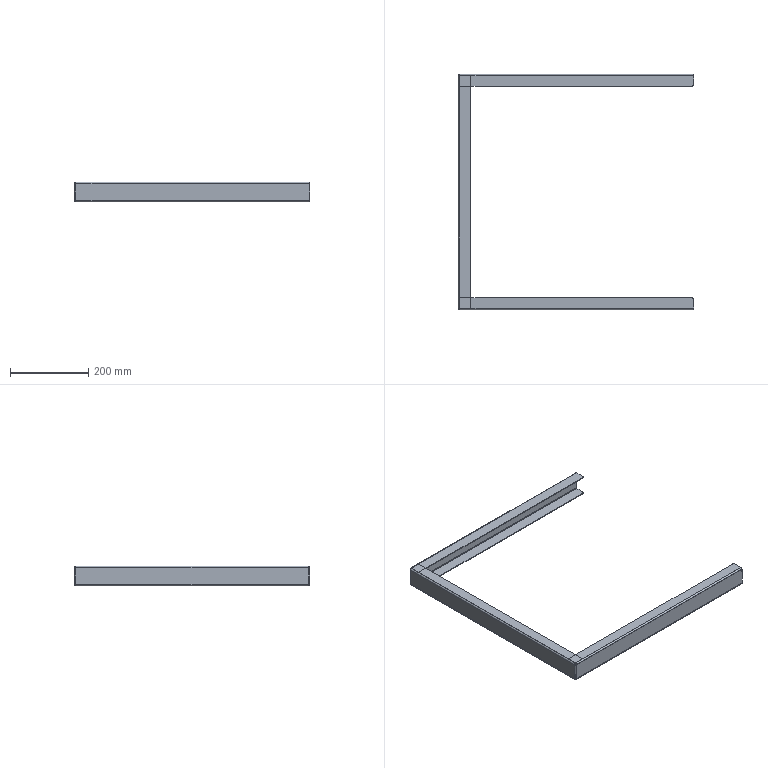Part | STEP file | 750038407 | 1 solid | 58 faces | box 600 x 600 x 51 mm | volume 373355 mm3 | plane 38 | cylinder 20 | commonest cylinder face diameters 4 x8 8 x8 10 x4
STEP:
#1=CARTESIAN_POINT('',(598.,298.,21.5));
#2=VERTEX_POINT('',#1);
#3=CARTESIAN_POINT('',(2.,298.,21.5));
#4=VERTEX_POINT('',#3);
#5=CARTESIAN_POINT('',(598.,298.,21.5));
#6=DIRECTION('',(-1.,0.,0.));
#7=VECTOR('',#6,1000.);
#8=LINE('',#5,#7);
#9=EDGE_CURVE('',#2,#4,#8,.T.);
#10=ORIENTED_EDGE('',*,*,#9,.T.);
#11=CARTESIAN_POINT('',(2.,298.,-21.5));
#12=VERTEX_POINT('',#11);
#13=CARTESIAN_POINT('',(2.,298.,21.5));
#14=DIRECTION('',(0.,0.,-1.));
#15=VECTOR('',#14,1000.);
#16=LINE('',#13,#15);
#17=EDGE_CURVE('',#4,#12,#16,.T.);
#18=ORIENTED_EDGE('',*,*,#17,.T.);
#19=CARTESIAN_POINT('',(598.,298.,-21.5));
#20=VERTEX_POINT('',#19);
#21=CARTESIAN_POINT('',(598.,298.,-21.5));
#22=DIRECTION('',(1.,0.,0.));
#23=VECTOR('',#22,1000.);
#24=LINE('',#21,#23);
#25=EDGE_CURVE('',#12,#20,#24,.T.);
#26=ORIENTED_EDGE('',*,*,#25,.T.);
#27=CARTESIAN_POINT('',(598.,298.,21.5));
#28=DIRECTION('',(0.,0.,1.));
#29=VECTOR('',#28,1000.);
#30=LINE('',#27,#29);
#31=EDGE_CURVE('',#20,#2,#30,.T.);
#32=ORIENTED_EDGE('',*,*,#31,.T.);
#33=EDGE_LOOP('',(#10,#18,#26,#32));
#34=FACE_OUTER_BOUND('',#33,.T.);
#35=CARTESIAN_POINT('',(598.,298.,21.5));
#36=DIRECTION('',(0.,-1.,0.));
#37=DIRECTION('',(0.,0.,-1.));
#38=AXIS2_PLACEMENT_3D('',#35,#36,#37);
#39=PLANE('',#38);
#40=ADVANCED_FACE('',(#34),#39,.T.);
#41=ORIENTED_EDGE('',*,*,#17,.F.);
#42=CARTESIAN_POINT('',(0.,296.,21.5));
#43=VERTEX_POINT('',#42);
#44=CARTESIAN_POINT('',(2.,296.,21.5));
#45=DIRECTION('',(0.,0.,-1.));
#46=DIRECTION('',(-1.,0.,0.));
#47=AXIS2_PLACEMENT_3D('',#44,#45,#46);
#48=CIRCLE('',#47,2.);
#49=EDGE_CURVE('',#43,#4,#48,.T.);
#50=ORIENTED_EDGE('',*,*,#49,.F.);
#51=CARTESIAN_POINT('',(0.,296.,-21.5));
#52=VERTEX_POINT('',#51);
#53=CARTESIAN_POINT('',(0.,296.,21.5));
#54=DIRECTION('',(0.,0.,1.));
#55=VECTOR('',#54,1000.);
#56=LINE('',#53,#55);
#57=EDGE_CURVE('',#52,#43,#56,.T.);
#58=ORIENTED_EDGE('',*,*,#57,.F.);
#59=CARTESIAN_POINT('',(2.,296.,-21.5));
#60=DIRECTION('',(0.,0.,1.));
#61=DIRECTION('',(-1.,0.,0.));
#62=AXIS2_PLACEMENT_3D('',#59,#60,#61);
#63=CIRCLE('',#62,2.);
#64=EDGE_CURVE('',#12,#52,#63,.T.);
#65=ORIENTED_EDGE('',*,*,#64,.F.);
#66=EDGE_LOOP('',(#41,#50,#58,#65));
#67=FACE_OUTER_BOUND('',#66,.T.);
#68=CARTESIAN_POINT('',(2.,296.,21.5));
#69=DIRECTION('',(0.,0.,-1.));
#70=DIRECTION('',(-1.,0.,0.));
#71=AXIS2_PLACEMENT_3D('',#68,#69,#70);
#72=CYLINDRICAL_SURFACE('',#71,2.);
#73=ADVANCED_FACE('',(#67),#72,.F.);
#74=ORIENTED_EDGE('',*,*,#9,.F.);
#75=CARTESIAN_POINT('',(598.,296.,23.5));
#76=VERTEX_POINT('',#75);
#77=CARTESIAN_POINT('',(598.,296.,21.5));
#78=DIRECTION('',(-1.,0.,0.));
#79=DIRECTION('',(0.,0.,1.));
#80=AXIS2_PLACEMENT_3D('',#77,#78,#79);
#81=CIRCLE('',#80,2.);
#82=EDGE_CURVE('',#76,#2,#81,.T.);
#83=ORIENTED_EDGE('',*,*,#82,.F.);
#84=CARTESIAN_POINT('',(2.,296.,23.5));
#85=VERTEX_POINT('',#84);
#86=CARTESIAN_POINT('',(598.,296.,23.5));
#87=DIRECTION('',(1.,0.,0.));
#88=VECTOR('',#87,1000.);
#89=LINE('',#86,#88);
#90=EDGE_CURVE('',#85,#76,#89,.T.);
#91=ORIENTED_EDGE('',*,*,#90,.F.);
#92=CARTESIAN_POINT('',(2.,296.,21.5));
#93=DIRECTION('',(1.,0.,0.));
#94=DIRECTION('',(0.,0.,1.));
#95=AXIS2_PLACEMENT_3D('',#92,#93,#94);
#96=CIRCLE('',#95,2.);
#97=EDGE_CURVE('',#4,#85,#96,.T.);
#98=ORIENTED_EDGE('',*,*,#97,.F.);
#99=EDGE_LOOP('',(#74,#83,#91,#98));
#100=FACE_OUTER_BOUND('',#99,.T.);
#101=CARTESIAN_POINT('',(598.,296.,21.5));
#102=DIRECTION('',(-1.,0.,0.));
#103=DIRECTION('',(0.,0.,1.));
#104=AXIS2_PLACEMENT_3D('',#101,#102,#103);
#105=CYLINDRICAL_SURFACE('',#104,2.);
#106=ADVANCED_FACE('',(#100),#105,.F.);
#107=CARTESIAN_POINT('',(598.,275.,-25.5));
#108=VERTEX_POINT('',#107);
#109=CARTESIAN_POINT('',(598.,275.,-23.5));
#110=VERTEX_POINT('',#109);
#111=CARTESIAN_POINT('',(598.,275.,21.5));
#112=DIRECTION('',(0.,0.,1.));
#113=VECTOR('',#112,1000.);
#114=LINE('',#111,#113);
#115=EDGE_CURVE('',#108,#110,#114,.T.);
#116=ORIENTED_EDGE('',*,*,#115,.F.);
#117=CARTESIAN_POINT('',(598.,296.,-25.5));
#118=VERTEX_POINT('',#117);
#119=CARTESIAN_POINT('',(598.,298.,-25.5));
#120=DIRECTION('',(0.,-1.,0.));
#121=VECTOR('',#120,1000.);
#122=LINE('',#119,#121);
#123=EDGE_CURVE('',#118,#108,#122,.T.);
#124=ORIENTED_EDGE('',*,*,#123,.F.);
#125=CARTESIAN_POINT('',(598.,300.,-21.5));
#126=VERTEX_POINT('',#125);
#127=CARTESIAN_POINT('',(598.,296.,-21.5));
#128=DIRECTION('',(-1.,0.,0.));
#129=DIRECTION('',(0.,0.,-1.));
#130=AXIS2_PLACEMENT_3D('',#127,#128,#129);
#131=CIRCLE('',#130,4.);
#132=EDGE_CURVE('',#126,#118,#131,.T.);
#133=ORIENTED_EDGE('',*,*,#132,.F.);
#134=CARTESIAN_POINT('',(598.,300.,21.5));
#135=VERTEX_POINT('',#134);
#136=CARTESIAN_POINT('',(598.,300.,21.5));
#137=DIRECTION('',(0.,0.,-1.));
#138=VECTOR('',#137,1000.);
#139=LINE('',#136,#138);
#140=EDGE_CURVE('',#135,#126,#139,.T.);
#141=ORIENTED_EDGE('',*,*,#140,.F.);
#142=CARTESIAN_POINT('',(598.,296.,25.5));
#143=VERTEX_POINT('',#142);
#144=CARTESIAN_POINT('',(598.,296.,21.5));
#145=DIRECTION('',(-1.,0.,0.));
#146=DIRECTION('',(0.,0.,1.));
#147=AXIS2_PLACEMENT_3D('',#144,#145,#146);
#148=CIRCLE('',#147,4.);
#149=EDGE_CURVE('',#143,#135,#148,.T.);
#150=ORIENTED_EDGE('',*,*,#149,.F.);
#151=CARTESIAN_POINT('',(598.,275.,25.5));
#152=VERTEX_POINT('',#151);
#153=CARTESIAN_POINT('',(598.,298.,25.5));
#154=DIRECTION('',(0.,1.,0.));
#155=VECTOR('',#154,1000.);
#156=LINE('',#153,#155);
#157=EDGE_CURVE('',#152,#143,#156,.T.);
#158=ORIENTED_EDGE('',*,*,#157,.F.);
#159=CARTESIAN_POINT('',(598.,275.,23.5));
#160=VERTEX_POINT('',#159);
#161=CARTESIAN_POINT('',(598.,275.,21.5));
#162=DIRECTION('',(0.,0.,1.));
#163=VECTOR('',#162,1000.);
#164=LINE('',#161,#163);
#165=EDGE_CURVE('',#160,#152,#164,.T.);
#166=ORIENTED_EDGE('',*,*,#165,.F.);
#167=CARTESIAN_POINT('',(598.,298.,23.5));
#168=DIRECTION('',(0.,-1.,0.));
#169=VECTOR('',#168,1000.);
#170=LINE('',#167,#169);
#171=EDGE_CURVE('',#76,#160,#170,.T.);
#172=ORIENTED_EDGE('',*,*,#171,.F.);
#173=ORIENTED_EDGE('',*,*,#82,.T.);
#174=ORIENTED_EDGE('',*,*,#31,.F.);
#175=CARTESIAN_POINT('',(598.,296.,-23.5));
#176=VERTEX_POINT('',#175);
#177=CARTESIAN_POINT('',(598.,296.,-21.5));
#178=DIRECTION('',(1.,0.,0.));
#179=DIRECTION('',(0.,0.,-1.));
#180=AXIS2_PLACEMENT_3D('',#177,#178,#179);
#181=CIRCLE('',#180,2.);
#182=EDGE_CURVE('',#176,#20,#181,.T.);
#183=ORIENTED_EDGE('',*,*,#182,.F.);
#184=CARTESIAN_POINT('',(598.,298.,-23.5));
#185=DIRECTION('',(0.,1.,0.));
#186=VECTOR('',#185,1000.);
#187=LINE('',#184,#186);
#188=EDGE_CURVE('',#110,#176,#187,.T.);
#189=ORIENTED_EDGE('',*,*,#188,.F.);
#190=EDGE_LOOP('',(#116,#124,#133,#141,#150,#158,#166,#172,#173,#174,#183,#189));
#191=FACE_OUTER_BOUND('',#190,.T.);
#192=CARTESIAN_POINT('',(598.,298.,21.5));
#193=DIRECTION('',(-1.,0.,0.));
#194=DIRECTION('',(0.,0.,1.));
#195=AXIS2_PLACEMENT_3D('',#192,#193,#194);
#196=PLANE('',#195);
#197=ADVANCED_FACE('',(#191),#196,.F.);
#198=ORIENTED_EDGE('',*,*,#25,.F.);
#199=CARTESIAN_POINT('',(2.,296.,-23.5));
#200=VERTEX_POINT('',#199);
#201=CARTESIAN_POINT('',(2.,296.,-21.5));
#202=DIRECTION('',(1.,0.,0.));
#203=DIRECTION('',(0.,0.,-1.));
#204=AXIS2_PLACEMENT_3D('',#201,#202,#203);
#205=CIRCLE('',#204,2.);
#206=EDGE_CURVE('',#200,#12,#205,.T.);
#207=ORIENTED_EDGE('',*,*,#206,.F.);
#208=CARTESIAN_POINT('',(2.,296.,-23.5));
#209=DIRECTION('',(-1.,0.,0.));
#210=VECTOR('',#209,1000.);
#211=LINE('',#208,#210);
#212=EDGE_CURVE('',#176,#200,#211,.T.);
#213=ORIENTED_EDGE('',*,*,#212,.F.);
#214=ORIENTED_EDGE('',*,*,#182,.T.);
#215=EDGE_LOOP('',(#198,#207,#213,#214));
#216=FACE_OUTER_BOUND('',#215,.T.);
#217=CARTESIAN_POINT('',(2.,296.,-21.5));
#218=DIRECTION('',(1.,0.,0.));
#219=DIRECTION('',(0.,0.,-1.));
#220=AXIS2_PLACEMENT_3D('',#217,#218,#219);
#221=CYLINDRICAL_SURFACE('',#220,2.);
#222=ADVANCED_FACE('',(#216),#221,.F.);
#223=CARTESIAN_POINT('',(-2.,296.,-21.5));
#224=VERTEX_POINT('',#223);
#225=CARTESIAN_POINT('',(598.,296.,-21.5));
#226=DIRECTION('',(1.,0.,0.));
#227=VECTOR('',#226,1000.);
#228=LINE('',#225,#227);
#229=EDGE_CURVE('',#224,#52,#228,.T.);
#230=ORIENTED_EDGE('',*,*,#229,.F.);
#231=CARTESIAN_POINT('',(2.,300.,-21.5));
#232=VERTEX_POINT('',#231);
#233=CARTESIAN_POINT('',(2.,296.,-21.5));
#234=DIRECTION('',(0.,0.,1.));
#235=DIRECTION('',(-1.,0.,0.));
#236=AXIS2_PLACEMENT_3D('',#233,#234,#235);
#237=CIRCLE('',#236,4.);
#238=EDGE_CURVE('',#232,#224,#237,.T.);
#239=ORIENTED_EDGE('',*,*,#238,.F.);
#240=CARTESIAN_POINT('',(2.,298.,-21.5));
#241=DIRECTION('',(0.,1.,0.));
#242=VECTOR('',#241,1000.);
#243=LINE('',#240,#242);
#244=EDGE_CURVE('',#12,#232,#243,.T.);
#245=ORIENTED_EDGE('',*,*,#244,.F.);
#246=ORIENTED_EDGE('',*,*,#64,.T.);
#247=EDGE_LOOP('',(#230,#239,#245,#246));
#248=FACE_OUTER_BOUND('',#247,.T.);
#249=CARTESIAN_POINT('',(598.,298.,-21.5));
#250=DIRECTION('',(0.,0.,1.));
#251=DIRECTION('',(1.,0.,0.));
#252=AXIS2_PLACEMENT_3D('',#249,#250,#251);
#253=PLANE('',#252);
#254=ADVANCED_FACE('',(#248),#253,.F.);
#255=CARTESIAN_POINT('',(2.,300.,21.5));
#256=VERTEX_POINT('',#255);
#257=CARTESIAN_POINT('',(2.,-298.,21.5));
#258=DIRECTION('',(0.,1.,0.));
#259=VECTOR('',#258,1000.);
#260=LINE('',#257,#259);
#261=EDGE_CURVE('',#4,#256,#260,.T.);
#262=ORIENTED_EDGE('',*,*,#261,.T.);
#263=CARTESIAN_POINT('',(-2.,296.,21.5));
#264=VERTEX_POINT('',#263);
#265=CARTESIAN_POINT('',(2.,296.,21.5));
#266=DIRECTION('',(0.,0.,1.));
#267=DIRECTION('',(-1.,0.,0.));
#268=AXIS2_PLACEMENT_3D('',#265,#266,#267);
#269=CIRCLE('',#268,4.);
#270=EDGE_CURVE('',#256,#264,#269,.T.);
#271=ORIENTED_EDGE('',*,*,#270,.T.);
#272=CARTESIAN_POINT('',(0.,296.,21.5));
#273=DIRECTION('',(1.,0.,0.));
#274=VECTOR('',#273,1000.);
#275=LINE('',#272,#274);
#276=EDGE_CURVE('',#264,#43,#275,.T.);
#277=ORIENTED_EDGE('',*,*,#276,.T.);
#278=ORIENTED_EDGE('',*,*,#49,.T.);
#279=EDGE_LOOP('',(#262,#271,#277,#278));
#280=FACE_OUTER_BOUND('',#279,.T.);
#281=CARTESIAN_POINT('',(0.,-298.,21.5));
#282=DIRECTION('',(0.,0.,1.));
#283=DIRECTION('',(1.,0.,0.));
#284=AXIS2_PLACEMENT_3D('',#281,#282,#283);
#285=PLANE('',#284);
#286=ADVANCED_FACE('',(#280),#285,.T.);
#287=CARTESIAN_POINT('',(0.,-296.,21.5));
#288=VERTEX_POINT('',#287);
#289=CARTESIAN_POINT('',(0.,298.,21.5));
#290=DIRECTION('',(0.,-1.,0.));
#291=VECTOR('',#290,1000.);
#292=LINE('',#289,#291);
#293=EDGE_CURVE('',#43,#288,#292,.T.);
#294=ORIENTED_EDGE('',*,*,#293,.T.);
#295=CARTESIAN_POINT('',(0.,-296.,-21.5));
#296=VERTEX_POINT('',#295);
#297=CARTESIAN_POINT('',(0.,-296.,21.5));
#298=DIRECTION('',(0.,0.,-1.));
#299=VECTOR('',#298,1000.);
#300=LINE('',#297,#299);
#301=EDGE_CURVE('',#288,#296,#300,.T.);
#302=ORIENTED_EDGE('',*,*,#301,.T.);
#303=CARTESIAN_POINT('',(0.,298.,-21.5));
#304=DIRECTION('',(0.,1.,0.));
#305=VECTOR('',#304,1000.);
#306=LINE('',#303,#305);
#307=EDGE_CURVE('',#296,#52,#306,.T.);
#308=ORIENTED_EDGE('',*,*,#307,.T.);
#309=ORIENTED_EDGE('',*,*,#57,.T.);
#310=EDGE_LOOP('',(#294,#302,#308,#309));
#311=FACE_OUTER_BOUND('',#310,.T.);
#312=CARTESIAN_POINT('',(0.,298.,21.5));
#313=DIRECTION('',(1.,0.,0.));
#314=DIRECTION('',(0.,0.,-1.));
#315=AXIS2_PLACEMENT_3D('',#312,#313,#314);
#316=PLANE('',#315);
#317=ADVANCED_FACE('',(#311),#316,.T.);
#318=CARTESIAN_POINT('',(2.,296.,25.5));
#319=VERTEX_POINT('',#318);
#320=CARTESIAN_POINT('',(2.,296.,21.5));
#321=DIRECTION('',(-1.,0.,0.));
#322=DIRECTION('',(0.,0.,1.));
#323=AXIS2_PLACEMENT_3D('',#320,#321,#322);
#324=CIRCLE('',#323,4.);
#325=EDGE_CURVE('',#319,#256,#324,.T.);
#326=ORIENTED_EDGE('',*,*,#325,.T.);
#327=ORIENTED_EDGE('',*,*,#261,.F.);
#328=ORIENTED_EDGE('',*,*,#97,.T.);
#329=CARTESIAN_POINT('',(2.,270.,23.5));
#330=VERTEX_POINT('',#329);
#331=CARTESIAN_POINT('',(2.,296.,23.5));
#332=DIRECTION('',(0.,-1.,0.));
#333=VECTOR('',#332,1000.);
#334=LINE('',#331,#333);
#335=EDGE_CURVE('',#85,#330,#334,.T.);
#336=ORIENTED_EDGE('',*,*,#335,.T.);
#337=CARTESIAN_POINT('',(2.,270.,25.5));
#338=VERTEX_POINT('',#337);
#339=CARTESIAN_POINT('',(2.,270.,21.5));
#340=DIRECTION('',(0.,0.,1.));
#341=VECTOR('',#340,1000.);
#342=LINE('',#339,#341);
#343=EDGE_CURVE('',#330,#338,#342,.T.);
#344=ORIENTED_EDGE('',*,*,#343,.T.);
#345=CARTESIAN_POINT('',(2.,296.,25.5));
#346=DIRECTION('',(0.,1.,0.));
#347=VECTOR('',#346,1000.);
#348=LINE('',#345,#347);
#349=EDGE_CURVE('',#338,#319,#348,.T.);
#350=ORIENTED_EDGE('',*,*,#349,.T.);
#351=EDGE_LOOP('',(#326,#327,#328,#336,#344,#350));
#352=FACE_OUTER_BOUND('',#351,.T.);
#353=CARTESIAN_POINT('',(2.,296.,21.5));
#354=DIRECTION('',(-1.,0.,0.));
#355=DIRECTION('',(0.,0.,1.));
#356=AXIS2_PLACEMENT_3D('',#353,#354,#355);
#357=PLANE('',#356);
#358=ADVANCED_FACE('',(#352),#357,.T.);
#359=ORIENTED_EDGE('',*,*,#335,.F.);
#360=ORIENTED_EDGE('',*,*,#90,.T.);
#361=ORIENTED_EDGE('',*,*,#171,.T.);
#362=CARTESIAN_POINT('',(593.,270.,23.5));
#363=VERTEX_POINT('',#362);
#364=CARTESIAN_POINT('',(593.,275.,23.5));
#365=DIRECTION('',(0.,0.,-1.));
#366=DIRECTION('',(1.,0.,0.));
#367=AXIS2_PLACEMENT_3D('',#364,#365,#366);
#368=CIRCLE('',#367,5.);
#369=EDGE_CURVE('',#160,#363,#368,.T.);
#370=ORIENTED_EDGE('',*,*,#369,.T.);
#371=CARTESIAN_POINT('',(598.,270.,23.5));
#372=DIRECTION('',(-1.,0.,0.));
#373=VECTOR('',#372,1000.);
#374=LINE('',#371,#373);
#375=EDGE_CURVE('',#363,#330,#374,.T.);
#376=ORIENTED_EDGE('',*,*,#375,.T.);
#377=EDGE_LOOP('',(#359,#360,#361,#370,#376));
#378=FACE_OUTER_BOUND('',#377,.T.);
#379=CARTESIAN_POINT('',(598.,296.,23.5));
#380=DIRECTION('',(0.,0.,-1.));
#381=DIRECTION('',(-1.,0.,0.));
#382=AXIS2_PLACEMENT_3D('',#379,#380,#381);
#383=PLANE('',#382);
#384=ADVANCED_FACE('',(#378),#383,.T.);
#385=ORIENTED_EDGE('',*,*,#212,.T.);
#386=CARTESIAN_POINT('',(2.,270.,-23.5));
#387=VERTEX_POINT('',#386);
#388=CARTESIAN_POINT('',(2.,296.,-23.5));
#389=DIRECTION('',(0.,-1.,0.));
#390=VECTOR('',#389,1000.);
#391=LINE('',#388,#390);
#392=EDGE_CURVE('',#200,#387,#391,.T.);
#393=ORIENTED_EDGE('',*,*,#392,.T.);
#394=CARTESIAN_POINT('',(593.,270.,-23.5));
#395=VERTEX_POINT('',#394);
#396=CARTESIAN_POINT('',(2.,270.,-23.5));
#397=DIRECTION('',(1.,0.,0.));
#398=VECTOR('',#397,1000.);
#399=LINE('',#396,#398);
#400=EDGE_CURVE('',#387,#395,#399,.T.);
#401=ORIENTED_EDGE('',*,*,#400,.T.);
#402=CARTESIAN_POINT('',(593.,275.,-23.5));
#403=DIRECTION('',(0.,0.,1.));
#404=DIRECTION('',(-1.,0.,0.));
#405=AXIS2_PLACEMENT_3D('',#402,#403,#404);
#406=CIRCLE('',#405,5.);
#407=EDGE_CURVE('',#395,#110,#406,.T.);
#408=ORIENTED_EDGE('',*,*,#407,.T.);
#409=ORIENTED_EDGE('',*,*,#188,.T.);
#410=EDGE_LOOP('',(#385,#393,#401,#408,#409));
#411=FACE_OUTER_BOUND('',#410,.T.);
#412=CARTESIAN_POINT('',(2.,296.,-23.5));
#413=DIRECTION('',(0.,0.,1.));
#414=DIRECTION('',(1.,0.,0.));
#415=AXIS2_PLACEMENT_3D('',#412,#413,#414);
#416=PLANE('',#415);
#417=ADVANCED_FACE('',(#411),#416,.T.);
#418=ORIENTED_EDGE('',*,*,#407,.F.);
#419=CARTESIAN_POINT('',(593.,270.,-25.5));
#420=VERTEX_POINT('',#419);
#421=CARTESIAN_POINT('',(593.,270.,-23.5));
#422=DIRECTION('',(0.,0.,-1.));
#423=VECTOR('',#422,1000.);
#424=LINE('',#421,#423);
#425=EDGE_CURVE('',#395,#420,#424,.T.);
#426=ORIENTED_EDGE('',*,*,#425,.T.);
#427=CARTESIAN_POINT('',(593.,275.,-25.5));
#428=DIRECTION('',(0.,0.,1.));
#429=DIRECTION('',(-1.,0.,0.));
#430=AXIS2_PLACEMENT_3D('',#427,#428,#429);
#431=CIRCLE('',#430,5.);
#432=EDGE_CURVE('',#420,#108,#431,.T.);
#433=ORIENTED_EDGE('',*,*,#432,.T.);
#434=ORIENTED_EDGE('',*,*,#115,.T.);
#435=EDGE_LOOP('',(#418,#426,#433,#434));
#436=FACE_OUTER_BOUND('',#435,.T.);
#437=CARTESIAN_POINT('',(593.,275.,-23.5));
#438=DIRECTION('',(0.,0.,-1.));
#439=DIRECTION('',(-1.,0.,0.));
#440=AXIS2_PLACEMENT_3D('',#437,#438,#439);
#441=CYLINDRICAL_SURFACE('',#440,5.);
#442=ADVANCED_FACE('',(#436),#441,.T.);
#443=ORIENTED_EDGE('',*,*,#432,.F.);
#444=CARTESIAN_POINT('',(2.,270.,-25.5));
#445=VERTEX_POINT('',#444);
#446=CARTESIAN_POINT('',(2.,270.,-25.5));
#447=DIRECTION('',(1.,0.,0.));
#448=VECTOR('',#447,1000.);
#449=LINE('',#446,#448);
#450=EDGE_CURVE('',#445,#420,#449,.T.);
#451=ORIENTED_EDGE('',*,*,#450,.F.);
#452=CARTESIAN_POINT('',(2.,296.,-25.5));
#453=VERTEX_POINT('',#452);
#454=CARTESIAN_POINT('',(2.,296.,-25.5));
#455=DIRECTION('',(0.,-1.,0.));
#456=VECTOR('',#455,1000.);
#457=LINE('',#454,#456);
#458=EDGE_CURVE('',#453,#445,#457,.T.);
#459=ORIENTED_EDGE('',*,*,#458,.F.);
#460=CARTESIAN_POINT('',(2.,296.,-25.5));
#461=DIRECTION('',(-1.,0.,0.));
#462=VECTOR('',#461,1000.);
#463=LINE('',#460,#462);
#464=EDGE_CURVE('',#118,#453,#463,.T.);
#465=ORIENTED_EDGE('',*,*,#464,.F.);
#466=ORIENTED_EDGE('',*,*,#123,.T.);
#467=EDGE_LOOP('',(#443,#451,#459,#465,#466));
#468=FACE_OUTER_BOUND('',#467,.T.);
#469=CARTESIAN_POINT('',(2.,296.,-25.5));
#470=DIRECTION('',(0.,0.,1.));
#471=DIRECTION('',(1.,0.,0.));
#472=AXIS2_PLACEMENT_3D('',#469,#470,#471);
#473=PLANE('',#472);
#474=ADVANCED_FACE('',(#468),#473,.F.);
#475=CARTESIAN_POINT('',(2.,296.,-21.5));
#476=DIRECTION('',(1.,0.,0.));
#477=DIRECTION('',(0.,0.,-1.));
#478=AXIS2_PLACEMENT_3D('',#475,#476,#477);
#479=CIRCLE('',#478,4.);
#480=EDGE_CURVE('',#453,#232,#479,.T.);
#481=ORIENTED_EDGE('',*,*,#480,.T.);
#482=CARTESIAN_POINT('',(2.,300.,-21.5));
#483=DIRECTION('',(1.,0.,0.));
#484=VECTOR('',#483,1000.);
#485=LINE('',#482,#484);
#486=EDGE_CURVE('',#232,#126,#485,.T.);
#487=ORIENTED_EDGE('',*,*,#486,.T.);
#488=ORIENTED_EDGE('',*,*,#132,.T.);
#489=ORIENTED_EDGE('',*,*,#464,.T.);
#490=EDGE_LOOP('',(#481,#487,#488,#489));
#491=FACE_OUTER_BOUND('',#490,.T.);
#492=CARTESIAN_POINT('',(2.,296.,-21.5));
#493=DIRECTION('',(1.,0.,0.));
#494=DIRECTION('',(0.,0.,-1.));
#495=AXIS2_PLACEMENT_3D('',#492,#493,#494);
#496=CYLINDRICAL_SURFACE('',#495,4.);
#497=ADVANCED_FACE('',(#491),#496,.T.);
#498=CARTESIAN_POINT('',(2.,300.,21.5));
#499=DIRECTION('',(0.,0.,-1.));
#500=VECTOR('',#499,1000.);
#501=LINE('',#498,#500);
#502=EDGE_CURVE('',#256,#232,#501,.T.);
#503=ORIENTED_EDGE('',*,*,#502,.F.);
#504=CARTESIAN_POINT('',(598.,300.,21.5));
#505=DIRECTION('',(-1.,0.,0.));
#506=VECTOR('',#505,1000.);
#507=LINE('',#504,#506);
#508=EDGE_CURVE('',#135,#256,#507,.T.);
#509=ORIENTED_EDGE('',*,*,#508,.F.);
#510=ORIENTED_EDGE('',*,*,#140,.T.);
#511=ORIENTED_EDGE('',*,*,#486,.F.);
#512=EDGE_LOOP('',(#503,#509,#510,#511));
#513=FACE_OUTER_BOUND('',#512,.T.);
#514=CARTESIAN_POINT('',(598.,300.,21.5));
#515=DIRECTION('',(0.,-1.,0.));
#516=DIRECTION('',(0.,0.,-1.));
#517=AXIS2_PLACEMENT_3D('',#514,#515,#516);
#518=PLANE('',#517);
#519=ADVANCED_FACE('',(#513),#518,.F.);
#520=ORIENTED_EDGE('',*,*,#149,.T.);
#521=ORIENTED_EDGE('',*,*,#508,.T.);
#522=ORIENTED_EDGE('',*,*,#325,.F.);
#523=CARTESIAN_POINT('',(598.,296.,25.5));
#524=DIRECTION('',(1.,0.,0.));
#525=VECTOR('',#524,1000.);
#526=LINE('',#523,#525);
#527=EDGE_CURVE('',#319,#143,#526,.T.);
#528=ORIENTED_EDGE('',*,*,#527,.T.);
#529=EDGE_LOOP('',(#520,#521,#522,#528));
#530=FACE_OUTER_BOUND('',#529,.T.);
#531=CARTESIAN_POINT('',(598.,296.,21.5));
#532=DIRECTION('',(-1.,0.,0.));
#533=DIRECTION('',(0.,0.,1.));
#534=AXIS2_PLACEMENT_3D('',#531,#532,#533);
#535=CYLINDRICAL_SURFACE('',#534,4.);
#536=ADVANCED_FACE('',(#530),#535,.T.);
#537=CARTESIAN_POINT('',(593.,270.,25.5));
#538=VERTEX_POINT('',#537);
#539=CARTESIAN_POINT('',(593.,275.,25.5));
#540=DIRECTION('',(0.,0.,-1.));
#541=DIRECTION('',(1.,0.,0.));
#542=AXIS2_PLACEMENT_3D('',#539,#540,#541);
#543=CIRCLE('',#542,5.);
#544=EDGE_CURVE('',#152,#538,#543,.T.);
#545=ORIENTED_EDGE('',*,*,#544,.F.);
#546=ORIENTED_EDGE('',*,*,#157,.T.);
#547=ORIENTED_EDGE('',*,*,#527,.F.);
#548=ORIENTED_EDGE('',*,*,#349,.F.);
#549=CARTESIAN_POINT('',(598.,270.,25.5));
#550=DIRECTION('',(-1.,0.,0.));
#551=VECTOR('',#550,1000.);
#552=LINE('',#549,#551);
#553=EDGE_CURVE('',#538,#338,#552,.T.);
#554=ORIENTED_EDGE('',*,*,#553,.F.);
#555=EDGE_LOOP('',(#545,#546,#547,#548,#554));
#556=FACE_OUTER_BOUND('',#555,.T.);
#557=CARTESIAN_POINT('',(598.,296.,25.5));
#558=DIRECTION('',(0.,0.,-1.));
#559=DIRECTION('',(-1.,0.,0.));
#560=AXIS2_PLACEMENT_3D('',#557,#558,#559);
#561=PLANE('',#560);
#562=ADVANCED_FACE('',(#556),#561,.F.);
#563=ORIENTED_EDGE('',*,*,#369,.F.);
#564=ORIENTED_EDGE('',*,*,#165,.T.);
#565=ORIENTED_EDGE('',*,*,#544,.T.);
#566=CARTESIAN_POINT('',(593.,270.,21.5));
#567=DIRECTION('',(0.,0.,-1.));
#568=VECTOR('',#567,1000.);
#569=LINE('',#566,#568);
#570=EDGE_CURVE('',#538,#363,#569,.T.);
#571=ORIENTED_EDGE('',*,*,#570,.T.);
#572=EDGE_LOOP('',(#563,#564,#565,#571));
#573=FACE_OUTER_BOUND('',#572,.T.);
#574=CARTESIAN_POINT('',(593.,275.,21.5));
#575=DIRECTION('',(0.,0.,1.));
#576=DIRECTION('',(1.,0.,0.));
#577=AXIS2_PLACEMENT_3D('',#574,#575,#576);
#578=CYLINDRICAL_SURFACE('',#577,5.);
#579=ADVANCED_FACE('',(#573),#578,.T.);
#580=ORIENTED_EDGE('',*,*,#458,.T.);
#581=CARTESIAN_POINT('',(2.,270.,-23.5));
#582=DIRECTION('',(0.,0.,1.));
#583=VECTOR('',#582,1000.);
#584=LINE('',#581,#583);
#585=EDGE_CURVE('',#445,#387,#584,.T.);
#586=ORIENTED_EDGE('',*,*,#585,.T.);
#587=ORIENTED_EDGE('',*,*,#392,.F.);
#588=ORIENTED_EDGE('',*,*,#206,.T.);
#589=ORIENTED_EDGE('',*,*,#244,.T.);
#590=ORIENTED_EDGE('',*,*,#480,.F.);
#591=EDGE_LOOP('',(#580,#586,#587,#588,#589,#590));
#592=FACE_OUTER_BOUND('',#591,.T.);
#593=CARTESIAN_POINT('',(2.,296.,-23.5));
#594=DIRECTION('',(-1.,0.,0.));
#595=DIRECTION('',(0.,0.,1.));
#596=AXIS2_PLACEMENT_3D('',#593,#594,#595);
#597=PLANE('',#596);
#598=ADVANCED_FACE('',(#592),#597,.T.);
#599=CARTESIAN_POINT('',(2.,296.,-25.5));
#600=VERTEX_POINT('',#599);
#601=CARTESIAN_POINT('',(2.,296.,-21.5));
#602=DIRECTION('',(0.,1.,0.));
#603=DIRECTION('',(0.,0.,1.));
#604=AXIS2_PLACEMENT_3D('',#601,#602,#603);
#605=CIRCLE('',#604,4.);
#606=EDGE_CURVE('',#600,#224,#605,.T.);
#607=ORIENTED_EDGE('',*,*,#606,.T.);
#608=ORIENTED_EDGE('',*,*,#229,.T.);
#609=CARTESIAN_POINT('',(2.,296.,-23.5));
#610=VERTEX_POINT('',#609);
#611=CARTESIAN_POINT('',(2.,296.,-21.5));
#612=DIRECTION('',(0.,-1.,0.));
#613=DIRECTION('',(0.,0.,1.));
#614=AXIS2_PLACEMENT_3D('',#611,#612,#613);
#615=CIRCLE('',#614,2.);
#616=EDGE_CURVE('',#52,#610,#615,.T.);
#617=ORIENTED_EDGE('',*,*,#616,.T.);
#618=CARTESIAN_POINT('',(28.,296.,-23.5));
#619=VERTEX_POINT('',#618);
#620=CARTESIAN_POINT('',(2.,296.,-23.5));
#621=DIRECTION('',(1.,0.,0.));
#622=VECTOR('',#621,1000.);
#623=LINE('',#620,#622);
#624=EDGE_CURVE('',#610,#619,#623,.T.);
#625=ORIENTED_EDGE('',*,*,#624,.T.);
#626=CARTESIAN_POINT('',(28.,296.,-25.5));
#627=VERTEX_POINT('',#626);
#628=CARTESIAN_POINT('',(28.,296.,-21.5));
#629=DIRECTION('',(0.,0.,-1.));
#630=VECTOR('',#629,1000.);
#631=LINE('',#628,#630);
#632=EDGE_CURVE('',#619,#627,#631,.T.);
#633=ORIENTED_EDGE('',*,*,#632,.T.);
#634=CARTESIAN_POINT('',(2.,296.,-25.5));
#635=DIRECTION('',(-1.,0.,0.));
#636=VECTOR('',#635,1000.);
#637=LINE('',#634,#636);
#638=EDGE_CURVE('',#627,#600,#637,.T.);
#639=ORIENTED_EDGE('',*,*,#638,.T.);
#640=EDGE_LOOP('',(#607,#608,#617,#625,#633,#639));
#641=FACE_OUTER_BOUND('',#640,.T.);
#642=CARTESIAN_POINT('',(2.,296.,-21.5));
#643=DIRECTION('',(0.,1.,0.));
#644=DIRECTION('',(0.,0.,1.));
#645=AXIS2_PLACEMENT_3D('',#642,#643,#644);
#646=PLANE('',#645);
#647=ADVANCED_FACE('',(#641),#646,.T.);
#648=ORIENTED_EDGE('',*,*,#270,.F.);
#649=ORIENTED_EDGE('',*,*,#502,.T.);
#650=ORIENTED_EDGE('',*,*,#238,.T.);
#651=CARTESIAN_POINT('',(-2.,296.,21.5));
#652=DIRECTION('',(0.,0.,1.));
#653=VECTOR('',#652,1000.);
#654=LINE('',#651,#653);
#655=EDGE_CURVE('',#224,#264,#654,.T.);
#656=ORIENTED_EDGE('',*,*,#655,.T.);
#657=EDGE_LOOP('',(#648,#649,#650,#656));
#658=FACE_OUTER_BOUND('',#657,.T.);
#659=CARTESIAN_POINT('',(2.,296.,21.5));
#660=DIRECTION('',(0.,0.,-1.));
#661=DIRECTION('',(-1.,0.,0.));
#662=AXIS2_PLACEMENT_3D('',#659,#660,#661);
#663=CYLINDRICAL_SURFACE('',#662,4.);
#664=ADVANCED_FACE('',(#658),#663,.T.);
#665=CARTESIAN_POINT('',(2.,296.,25.5));
#666=VERTEX_POINT('',#665);
#667=CARTESIAN_POINT('',(28.,296.,25.5));
#668=VERTEX_POINT('',#667);
#669=CARTESIAN_POINT('',(2.,296.,25.5));
#670=DIRECTION('',(1.,0.,0.));
#671=VECTOR('',#670,1000.);
#672=LINE('',#669,#671);
#673=EDGE_CURVE('',#666,#668,#672,.T.);
#674=ORIENTED_EDGE('',*,*,#673,.T.);
#675=CARTESIAN_POINT('',(28.,296.,23.5));
#676=VERTEX_POINT('',#675);
#677=CARTESIAN_POINT('',(28.,296.,23.5));
#678=DIRECTION('',(0.,0.,-1.));
#679=VECTOR('',#678,1000.);
#680=LINE('',#677,#679);
#681=EDGE_CURVE('',#668,#676,#680,.T.);
#682=ORIENTED_EDGE('',*,*,#681,.T.);
#683=CARTESIAN_POINT('',(2.,296.,23.5));
#684=VERTEX_POINT('',#683);
#685=CARTESIAN_POINT('',(2.,296.,23.5));
#686=DIRECTION('',(-1.,0.,0.));
#687=VECTOR('',#686,1000.);
#688=LINE('',#685,#687);
#689=EDGE_CURVE('',#676,#684,#688,.T.);
#690=ORIENTED_EDGE('',*,*,#689,.T.);
#691=CARTESIAN_POINT('',(2.,296.,21.5));
#692=DIRECTION('',(0.,-1.,0.));
#693=DIRECTION('',(0.,0.,-1.));
#694=AXIS2_PLACEMENT_3D('',#691,#692,#693);
#695=CIRCLE('',#694,2.);
#696=EDGE_CURVE('',#684,#43,#695,.T.);
#697=ORIENTED_EDGE('',*,*,#696,.T.);
#698=ORIENTED_EDGE('',*,*,#276,.F.);
#699=CARTESIAN_POINT('',(2.,296.,21.5));
#700=DIRECTION('',(0.,1.,0.));
#701=DIRECTION('',(0.,0.,-1.));
#702=AXIS2_PLACEMENT_3D('',#699,#700,#701);
#703=CIRCLE('',#702,4.);
#704=EDGE_CURVE('',#264,#666,#703,.T.);
#705=ORIENTED_EDGE('',*,*,#704,.T.);
#706=EDGE_LOOP('',(#674,#682,#690,#697,#698,#705));
#707=FACE_OUTER_BOUND('',#706,.T.);
#708=CARTESIAN_POINT('',(2.,296.,23.5));
#709=DIRECTION('',(0.,1.,0.));
#710=DIRECTION('',(0.,0.,1.));
#711=AXIS2_PLACEMENT_3D('',#708,#709,#710);
#712=PLANE('',#711);
#713=ADVANCED_FACE('',(#707),#712,.T.);
#714=ORIENTED_EDGE('',*,*,#301,.F.);
#715=CARTESIAN_POINT('',(2.,-298.,21.5));
#716=VERTEX_POINT('',#715);
#717=CARTESIAN_POINT('',(2.,-296.,21.5));
#718=DIRECTION('',(0.,0.,-1.));
#719=DIRECTION('',(-1.,0.,0.));
#720=AXIS2_PLACEMENT_3D('',#717,#718,#719);
#721=CIRCLE('',#720,2.);
#722=EDGE_CURVE('',#716,#288,#721,.T.);
#723=ORIENTED_EDGE('',*,*,#722,.F.);
#724=CARTESIAN_POINT('',(2.,-298.,-21.5));
#725=VERTEX_POINT('',#724);
#726=CARTESIAN_POINT('',(2.,-298.,21.5));
#727=DIRECTION('',(0.,0.,1.));
#728=VECTOR('',#727,1000.);
#729=LINE('',#726,#728);
#730=EDGE_CURVE('',#725,#716,#729,.T.);
#731=ORIENTED_EDGE('',*,*,#730,.F.);
#732=CARTESIAN_POINT('',(2.,-296.,-21.5));
#733=DIRECTION('',(0.,0.,1.));
#734=DIRECTION('',(-1.,0.,0.));
#735=AXIS2_PLACEMENT_3D('',#732,#733,#734);
#736=CIRCLE('',#735,2.);
#737=EDGE_CURVE('',#296,#725,#736,.T.);
#738=ORIENTED_EDGE('',*,*,#737,.F.);
#739=EDGE_LOOP('',(#714,#723,#731,#738));
#740=FACE_OUTER_BOUND('',#739,.T.);
#741=CARTESIAN_POINT('',(2.,-296.,21.5));
#742=DIRECTION('',(0.,0.,-1.));
#743=DIRECTION('',(-1.,0.,0.));
#744=AXIS2_PLACEMENT_3D('',#741,#742,#743);
#745=CYLINDRICAL_SURFACE('',#744,2.);
#746=ADVANCED_FACE('',(#740),#745,.F.);
#747=ORIENTED_EDGE('',*,*,#293,.F.);
#748=ORIENTED_EDGE('',*,*,#696,.F.);
#749=CARTESIAN_POINT('',(2.,-296.,23.5));
#750=VERTEX_POINT('',#749);
#751=CARTESIAN_POINT('',(2.,296.,23.5));
#752=DIRECTION('',(0.,1.,0.));
#753=VECTOR('',#752,1000.);
#754=LINE('',#751,#753);
#755=EDGE_CURVE('',#750,#684,#754,.T.);
#756=ORIENTED_EDGE('',*,*,#755,.F.);
#757=CARTESIAN_POINT('',(2.,-296.,21.5));
#758=DIRECTION('',(0.,1.,0.));
#759=DIRECTION('',(0.,0.,-1.));
#760=AXIS2_PLACEMENT_3D('',#757,#758,#759);
#761=CIRCLE('',#760,2.);
#762=EDGE_CURVE('',#288,#750,#761,.T.);
#763=ORIENTED_EDGE('',*,*,#762,.F.);
#764=EDGE_LOOP('',(#747,#748,#756,#763));
#765=FACE_OUTER_BOUND('',#764,.T.);
#766=CARTESIAN_POINT('',(2.,296.,21.5));
#767=DIRECTION('',(0.,-1.,0.));
#768=DIRECTION('',(0.,0.,-1.));
#769=AXIS2_PLACEMENT_3D('',#766,#767,#768);
#770=CYLINDRICAL_SURFACE('',#769,2.);
#771=ADVANCED_FACE('',(#765),#770,.F.);
#772=ORIENTED_EDGE('',*,*,#307,.F.);
#773=CARTESIAN_POINT('',(2.,-296.,-23.5));
#774=VERTEX_POINT('',#773);
#775=CARTESIAN_POINT('',(2.,-296.,-21.5));
#776=DIRECTION('',(0.,1.,0.));
#777=DIRECTION('',(0.,0.,1.));
#778=AXIS2_PLACEMENT_3D('',#775,#776,#777);
#779=CIRCLE('',#778,2.);
#780=EDGE_CURVE('',#774,#296,#779,.T.);
#781=ORIENTED_EDGE('',*,*,#780,.F.);
#782=CARTESIAN_POINT('',(2.,-296.,-23.5));
#783=DIRECTION('',(0.,-1.,0.));
#784=VECTOR('',#783,1000.);
#785=LINE('',#782,#784);
#786=EDGE_CURVE('',#610,#774,#785,.T.);
#787=ORIENTED_EDGE('',*,*,#786,.F.);
#788=ORIENTED_EDGE('',*,*,#616,.F.);
#789=EDGE_LOOP('',(#772,#781,#787,#788));
#790=FACE_OUTER_BOUND('',#789,.T.);
#791=CARTESIAN_POINT('',(2.,-296.,-21.5));
#792=DIRECTION('',(0.,1.,0.));
#793=DIRECTION('',(0.,0.,1.));
#794=AXIS2_PLACEMENT_3D('',#791,#792,#793);
#795=CYLINDRICAL_SURFACE('',#794,2.);
#796=ADVANCED_FACE('',(#790),#795,.F.);
#797=ORIENTED_EDGE('',*,*,#553,.T.);
#798=ORIENTED_EDGE('',*,*,#343,.F.);
#799=ORIENTED_EDGE('',*,*,#375,.F.);
#800=ORIENTED_EDGE('',*,*,#570,.F.);
#801=EDGE_LOOP('',(#797,#798,#799,#800));
#802=FACE_OUTER_BOUND('',#801,.T.);
#803=CARTESIAN_POINT('',(598.,270.,23.5));
#804=DIRECTION('',(0.,-1.,0.));
#805=DIRECTION('',(0.,0.,-1.));
#806=AXIS2_PLACEMENT_3D('',#803,#804,#805);
#807=PLANE('',#806);
#808=ADVANCED_FACE('',(#802),#807,.T.);
#809=ORIENTED_EDGE('',*,*,#400,.F.);
#810=ORIENTED_EDGE('',*,*,#585,.F.);
#811=ORIENTED_EDGE('',*,*,#450,.T.);
#812=ORIENTED_EDGE('',*,*,#425,.F.);
#813=EDGE_LOOP('',(#809,#810,#811,#812));
#814=FACE_OUTER_BOUND('',#813,.T.);
#815=CARTESIAN_POINT('',(2.,270.,-23.5));
#816=DIRECTION('',(0.,-1.,0.));
#817=DIRECTION('',(0.,0.,-1.));
#818=AXIS2_PLACEMENT_3D('',#815,#816,#817);
#819=PLANE('',#818);
#820=ADVANCED_FACE('',(#814),#819,.T.);
#821=CARTESIAN_POINT('',(2.,-296.,-25.5));
#822=VERTEX_POINT('',#821);
#823=CARTESIAN_POINT('',(-2.,-296.,-21.5));
#824=VERTEX_POINT('',#823);
#825=CARTESIAN_POINT('',(2.,-296.,-21.5));
#826=DIRECTION('',(0.,1.,0.));
#827=DIRECTION('',(0.,0.,1.));
#828=AXIS2_PLACEMENT_3D('',#825,#826,#827);
#829=CIRCLE('',#828,4.);
#830=EDGE_CURVE('',#822,#824,#829,.T.);
#831=ORIENTED_EDGE('',*,*,#830,.T.);
#832=CARTESIAN_POINT('',(-2.,-296.,-21.5));
#833=DIRECTION('',(0.,1.,0.));
#834=VECTOR('',#833,1000.);
#835=LINE('',#832,#834);
#836=EDGE_CURVE('',#824,#224,#835,.T.);
#837=ORIENTED_EDGE('',*,*,#836,.T.);
#838=ORIENTED_EDGE('',*,*,#606,.F.);
#839=CARTESIAN_POINT('',(2.,-296.,-25.5));
#840=DIRECTION('',(0.,-1.,0.));
#841=VECTOR('',#840,1000.);
#842=LINE('',#839,#841);
#843=EDGE_CURVE('',#600,#822,#842,.T.);
#844=ORIENTED_EDGE('',*,*,#843,.T.);
#845=EDGE_LOOP('',(#831,#837,#838,#844));
#846=FACE_OUTER_BOUND('',#845,.T.);
#847=CARTESIAN_POINT('',(2.,-296.,-21.5));
#848=DIRECTION('',(0.,1.,0.));
#849=DIRECTION('',(0.,0.,1.));
#850=AXIS2_PLACEMENT_3D('',#847,#848,#849);
#851=CYLINDRICAL_SURFACE('',#850,4.);
#852=ADVANCED_FACE('',(#846),#851,.T.);
#853=CARTESIAN_POINT('',(28.,-296.,-25.5));
#854=VERTEX_POINT('',#853);
#855=CARTESIAN_POINT('',(28.,-296.,-25.5));
#856=DIRECTION('',(0.,1.,0.));
#857=VECTOR('',#856,1000.);
#858=LINE('',#855,#857);
#859=EDGE_CURVE('',#854,#627,#858,.T.);
#860=ORIENTED_EDGE('',*,*,#859,.F.);
#861=CARTESIAN_POINT('',(2.,-296.,-25.5));
#862=DIRECTION('',(1.,0.,0.));
#863=VECTOR('',#862,1000.);
#864=LINE('',#861,#863);
#865=EDGE_CURVE('',#822,#854,#864,.T.);
#866=ORIENTED_EDGE('',*,*,#865,.F.);
#867=ORIENTED_EDGE('',*,*,#843,.F.);
#868=ORIENTED_EDGE('',*,*,#638,.F.);
#869=EDGE_LOOP('',(#860,#866,#867,#868));
#870=FACE_OUTER_BOUND('',#869,.T.);
#871=CARTESIAN_POINT('',(2.,-296.,-25.5));
#872=DIRECTION('',(0.,0.,1.));
#873=DIRECTION('',(1.,0.,0.));
#874=AXIS2_PLACEMENT_3D('',#871,#872,#873);
#875=PLANE('',#874);
#876=ADVANCED_FACE('',(#870),#875,.F.);
#877=ORIENTED_EDGE('',*,*,#632,.F.);
#878=CARTESIAN_POINT('',(28.,-296.,-23.5));
#879=VERTEX_POINT('',#878);
#880=CARTESIAN_POINT('',(28.,-296.,-23.5));
#881=DIRECTION('',(0.,-1.,0.));
#882=VECTOR('',#881,1000.);
#883=LINE('',#880,#882);
#884=EDGE_CURVE('',#619,#879,#883,.T.);
#885=ORIENTED_EDGE('',*,*,#884,.T.);
#886=CARTESIAN_POINT('',(28.,-296.,-23.5));
#887=DIRECTION('',(0.,0.,-1.));
#888=VECTOR('',#887,1000.);
#889=LINE('',#886,#888);
#890=EDGE_CURVE('',#879,#854,#889,.T.);
#891=ORIENTED_EDGE('',*,*,#890,.T.);
#892=ORIENTED_EDGE('',*,*,#859,.T.);
#893=EDGE_LOOP('',(#877,#885,#891,#892));
#894=FACE_OUTER_BOUND('',#893,.T.);
#895=CARTESIAN_POINT('',(28.,-296.,-23.5));
#896=DIRECTION('',(1.,0.,0.));
#897=DIRECTION('',(0.,0.,-1.));
#898=AXIS2_PLACEMENT_3D('',#895,#896,#897);
#899=PLANE('',#898);
#900=ADVANCED_FACE('',(#894),#899,.T.);
#901=CARTESIAN_POINT('',(2.,-296.,-23.5));
#902=DIRECTION('',(1.,0.,0.));
#903=VECTOR('',#902,1000.);
#904=LINE('',#901,#903);
#905=EDGE_CURVE('',#774,#879,#904,.T.);
#906=ORIENTED_EDGE('',*,*,#905,.T.);
#907=ORIENTED_EDGE('',*,*,#884,.F.);
#908=ORIENTED_EDGE('',*,*,#624,.F.);
#909=ORIENTED_EDGE('',*,*,#786,.T.);
#910=EDGE_LOOP('',(#906,#907,#908,#909));
#911=FACE_OUTER_BOUND('',#910,.T.);
#912=CARTESIAN_POINT('',(2.,-296.,-23.5));
#913=DIRECTION('',(0.,0.,1.));
#914=DIRECTION('',(1.,0.,0.));
#915=AXIS2_PLACEMENT_3D('',#912,#913,#914);
#916=PLANE('',#915);
#917=ADVANCED_FACE('',(#911),#916,.T.);
#918=CARTESIAN_POINT('',(-2.,-296.,21.5));
#919=VERTEX_POINT('',#918);
#920=CARTESIAN_POINT('',(-2.,-296.,21.5));
#921=DIRECTION('',(0.,0.,-1.));
#922=VECTOR('',#921,1000.);
#923=LINE('',#920,#922);
#924=EDGE_CURVE('',#919,#824,#923,.T.);
#925=ORIENTED_EDGE('',*,*,#924,.F.);
#926=CARTESIAN_POINT('',(-2.,298.,21.5));
#927=DIRECTION('',(0.,-1.,0.));
#928=VECTOR('',#927,1000.);
#929=LINE('',#926,#928);
#930=EDGE_CURVE('',#264,#919,#929,.T.);
#931=ORIENTED_EDGE('',*,*,#930,.F.);
#932=ORIENTED_EDGE('',*,*,#655,.F.);
#933=ORIENTED_EDGE('',*,*,#836,.F.);
#934=EDGE_LOOP('',(#925,#931,#932,#933));
#935=FACE_OUTER_BOUND('',#934,.T.);
#936=CARTESIAN_POINT('',(-2.,298.,21.5));
#937=DIRECTION('',(1.,0.,0.));
#938=DIRECTION('',(0.,0.,-1.));
#939=AXIS2_PLACEMENT_3D('',#936,#937,#938);
#940=PLANE('',#939);
#941=ADVANCED_FACE('',(#935),#940,.F.);
#942=CARTESIAN_POINT('',(28.,-296.,25.5));
#943=VERTEX_POINT('',#942);
#944=CARTESIAN_POINT('',(28.,-296.,23.5));
#945=VERTEX_POINT('',#944);
#946=CARTESIAN_POINT('',(28.,-296.,23.5));
#947=DIRECTION('',(0.,0.,-1.));
#948=VECTOR('',#947,1000.);
#949=LINE('',#946,#948);
#950=EDGE_CURVE('',#943,#945,#949,.T.);
#951=ORIENTED_EDGE('',*,*,#950,.T.);
#952=CARTESIAN_POINT('',(28.,296.,23.5));
#953=DIRECTION('',(0.,1.,0.));
#954=VECTOR('',#953,1000.);
#955=LINE('',#952,#954);
#956=EDGE_CURVE('',#945,#676,#955,.T.);
#957=ORIENTED_EDGE('',*,*,#956,.T.);
#958=ORIENTED_EDGE('',*,*,#681,.F.);
#959=CARTESIAN_POINT('',(28.,296.,25.5));
#960=DIRECTION('',(0.,-1.,0.));
#961=VECTOR('',#960,1000.);
#962=LINE('',#959,#961);
#963=EDGE_CURVE('',#668,#943,#962,.T.);
#964=ORIENTED_EDGE('',*,*,#963,.T.);
#965=EDGE_LOOP('',(#951,#957,#958,#964));
#966=FACE_OUTER_BOUND('',#965,.T.);
#967=CARTESIAN_POINT('',(28.,296.,23.5));
#968=DIRECTION('',(1.,0.,0.));
#969=DIRECTION('',(0.,0.,-1.));
#970=AXIS2_PLACEMENT_3D('',#967,#968,#969);
#971=PLANE('',#970);
#972=ADVANCED_FACE('',(#966),#971,.T.);
#973=ORIENTED_EDGE('',*,*,#963,.F.);
#974=ORIENTED_EDGE('',*,*,#673,.F.);
#975=CARTESIAN_POINT('',(2.,-296.,25.5));
#976=VERTEX_POINT('',#975);
#977=CARTESIAN_POINT('',(2.,296.,25.5));
#978=DIRECTION('',(0.,1.,0.));
#979=VECTOR('',#978,1000.);
#980=LINE('',#977,#979);
#981=EDGE_CURVE('',#976,#666,#980,.T.);
#982=ORIENTED_EDGE('',*,*,#981,.F.);
#983=CARTESIAN_POINT('',(2.,-296.,25.5));
#984=DIRECTION('',(-1.,0.,0.));
#985=VECTOR('',#984,1000.);
#986=LINE('',#983,#985);
#987=EDGE_CURVE('',#943,#976,#986,.T.);
#988=ORIENTED_EDGE('',*,*,#987,.F.);
#989=EDGE_LOOP('',(#973,#974,#982,#988));
#990=FACE_OUTER_BOUND('',#989,.T.);
#991=CARTESIAN_POINT('',(2.,296.,25.5));
#992=DIRECTION('',(0.,0.,-1.));
#993=DIRECTION('',(-1.,0.,0.));
#994=AXIS2_PLACEMENT_3D('',#991,#992,#993);
#995=PLANE('',#994);
#996=ADVANCED_FACE('',(#990),#995,.F.);
#997=ORIENTED_EDGE('',*,*,#704,.F.);
#998=ORIENTED_EDGE('',*,*,#930,.T.);
#999=CARTESIAN_POINT('',(2.,-296.,21.5));
#1000=DIRECTION('',(0.,1.,0.));
#1001=DIRECTION('',(0.,0.,-1.));
#1002=AXIS2_PLACEMENT_3D('',#999,#1000,#1001);
#1003=CIRCLE('',#1002,4.);
#1004=EDGE_CURVE('',#919,#976,#1003,.T.);
#1005=ORIENTED_EDGE('',*,*,#1004,.T.);
#1006=ORIENTED_EDGE('',*,*,#981,.T.);
#1007=EDGE_LOOP('',(#997,#998,#1005,#1006));
#1008=FACE_OUTER_BOUND('',#1007,.T.);
#1009=CARTESIAN_POINT('',(2.,296.,21.5));
#1010=DIRECTION('',(0.,-1.,0.));
#1011=DIRECTION('',(0.,0.,-1.));
#1012=AXIS2_PLACEMENT_3D('',#1009,#1010,#1011);
#1013=CYLINDRICAL_SURFACE('',#1012,4.);
#1014=ADVANCED_FACE('',(#1008),#1013,.T.);
#1015=ORIENTED_EDGE('',*,*,#689,.F.);
#1016=ORIENTED_EDGE('',*,*,#956,.F.);
#1017=CARTESIAN_POINT('',(2.,-296.,23.5));
#1018=DIRECTION('',(-1.,0.,0.));
#1019=VECTOR('',#1018,1000.);
#1020=LINE('',#1017,#1019);
#1021=EDGE_CURVE('',#945,#750,#1020,.T.);
#1022=ORIENTED_EDGE('',*,*,#1021,.T.);
#1023=ORIENTED_EDGE('',*,*,#755,.T.);
#1024=EDGE_LOOP('',(#1015,#1016,#1022,#1023));
#1025=FACE_OUTER_BOUND('',#1024,.T.);
#1026=CARTESIAN_POINT('',(2.,296.,23.5));
#1027=DIRECTION('',(0.,0.,-1.));
#1028=DIRECTION('',(-1.,0.,0.));
#1029=AXIS2_PLACEMENT_3D('',#1026,#1027,#1028);
#1030=PLANE('',#1029);
#1031=ADVANCED_FACE('',(#1025),#1030,.T.);
#1032=CARTESIAN_POINT('',(2.,-300.,-21.5));
#1033=VERTEX_POINT('',#1032);
#1034=CARTESIAN_POINT('',(2.,298.,-21.5));
#1035=DIRECTION('',(0.,1.,0.));
#1036=VECTOR('',#1035,1000.);
#1037=LINE('',#1034,#1036);
#1038=EDGE_CURVE('',#1033,#725,#1037,.T.);
#1039=ORIENTED_EDGE('',*,*,#1038,.F.);
#1040=CARTESIAN_POINT('',(2.,-296.,-21.5));
#1041=DIRECTION('',(0.,0.,1.));
#1042=DIRECTION('',(-1.,0.,0.));
#1043=AXIS2_PLACEMENT_3D('',#1040,#1041,#1042);
#1044=CIRCLE('',#1043,4.);
#1045=EDGE_CURVE('',#824,#1033,#1044,.T.);
#1046=ORIENTED_EDGE('',*,*,#1045,.F.);
#1047=CARTESIAN_POINT('',(598.,-296.,-21.5));
#1048=DIRECTION('',(-1.,0.,0.));
#1049=VECTOR('',#1048,1000.);
#1050=LINE('',#1047,#1049);
#1051=EDGE_CURVE('',#296,#824,#1050,.T.);
#1052=ORIENTED_EDGE('',*,*,#1051,.F.);
#1053=ORIENTED_EDGE('',*,*,#737,.T.);
#1054=EDGE_LOOP('',(#1039,#1046,#1052,#1053));
#1055=FACE_OUTER_BOUND('',#1054,.T.);
#1056=CARTESIAN_POINT('',(598.,298.,-21.5));
#1057=DIRECTION('',(0.,0.,1.));
#1058=DIRECTION('',(1.,0.,0.));
#1059=AXIS2_PLACEMENT_3D('',#1056,#1057,#1058);
#1060=PLANE('',#1059);
#1061=ADVANCED_FACE('',(#1055),#1060,.F.);
#1062=CARTESIAN_POINT('',(0.,-296.,21.5));
#1063=DIRECTION('',(-1.,0.,0.));
#1064=VECTOR('',#1063,1000.);
#1065=LINE('',#1062,#1064);
#1066=EDGE_CURVE('',#288,#919,#1065,.T.);
#1067=ORIENTED_EDGE('',*,*,#1066,.T.);
#1068=CARTESIAN_POINT('',(2.,-300.,21.5));
#1069=VERTEX_POINT('',#1068);
#1070=CARTESIAN_POINT('',(2.,-296.,21.5));
#1071=DIRECTION('',(0.,0.,1.));
#1072=DIRECTION('',(-1.,0.,0.));
#1073=AXIS2_PLACEMENT_3D('',#1070,#1071,#1072);
#1074=CIRCLE('',#1073,4.);
#1075=EDGE_CURVE('',#919,#1069,#1074,.T.);
#1076=ORIENTED_EDGE('',*,*,#1075,.T.);
#1077=CARTESIAN_POINT('',(2.,-298.,21.5));
#1078=DIRECTION('',(0.,1.,0.));
#1079=VECTOR('',#1078,1000.);
#1080=LINE('',#1077,#1079);
#1081=EDGE_CURVE('',#1069,#716,#1080,.T.);
#1082=ORIENTED_EDGE('',*,*,#1081,.T.);
#1083=ORIENTED_EDGE('',*,*,#722,.T.);
#1084=EDGE_LOOP('',(#1067,#1076,#1082,#1083));
#1085=FACE_OUTER_BOUND('',#1084,.T.);
#1086=CARTESIAN_POINT('',(0.,-298.,21.5));
#1087=DIRECTION('',(0.,0.,1.));
#1088=DIRECTION('',(1.,0.,0.));
#1089=AXIS2_PLACEMENT_3D('',#1086,#1087,#1088);
#1090=PLANE('',#1089);
#1091=ADVANCED_FACE('',(#1085),#1090,.T.);
#1092=CARTESIAN_POINT('',(598.,-298.,21.5));
#1093=VERTEX_POINT('',#1092);
#1094=CARTESIAN_POINT('',(0.,-298.,21.5));
#1095=DIRECTION('',(1.,0.,0.));
#1096=VECTOR('',#1095,1000.);
#1097=LINE('',#1094,#1096);
#1098=EDGE_CURVE('',#716,#1093,#1097,.T.);
#1099=ORIENTED_EDGE('',*,*,#1098,.T.);
#1100=CARTESIAN_POINT('',(598.,-298.,-21.5));
#1101=VERTEX_POINT('',#1100);
#1102=CARTESIAN_POINT('',(598.,-298.,21.5));
#1103=DIRECTION('',(0.,0.,-1.));
#1104=VECTOR('',#1103,1000.);
#1105=LINE('',#1102,#1104);
#1106=EDGE_CURVE('',#1093,#1101,#1105,.T.);
#1107=ORIENTED_EDGE('',*,*,#1106,.T.);
#1108=CARTESIAN_POINT('',(0.,-298.,-21.5));
#1109=DIRECTION('',(-1.,0.,0.));
#1110=VECTOR('',#1109,1000.);
#1111=LINE('',#1108,#1110);
#1112=EDGE_CURVE('',#1101,#725,#1111,.T.);
#1113=ORIENTED_EDGE('',*,*,#1112,.T.);
#1114=ORIENTED_EDGE('',*,*,#730,.T.);
#1115=EDGE_LOOP('',(#1099,#1107,#1113,#1114));
#1116=FACE_OUTER_BOUND('',#1115,.T.);
#1117=CARTESIAN_POINT('',(0.,-298.,21.5));
#1118=DIRECTION('',(0.,1.,0.));
#1119=DIRECTION('',(0.,0.,1.));
#1120=AXIS2_PLACEMENT_3D('',#1117,#1118,#1119);
#1121=PLANE('',#1120);
#1122=ADVANCED_FACE('',(#1116),#1121,.T.);
#1123=ORIENTED_EDGE('',*,*,#1004,.F.);
#1124=ORIENTED_EDGE('',*,*,#1066,.F.);
#1125=ORIENTED_EDGE('',*,*,#762,.T.);
#1126=ORIENTED_EDGE('',*,*,#1021,.F.);
#1127=ORIENTED_EDGE('',*,*,#950,.F.);
#1128=ORIENTED_EDGE('',*,*,#987,.T.);
#1129=EDGE_LOOP('',(#1123,#1124,#1125,#1126,#1127,#1128));
#1130=FACE_OUTER_BOUND('',#1129,.T.);
#1131=CARTESIAN_POINT('',(2.,-296.,21.5));
#1132=DIRECTION('',(0.,-1.,0.));
#1133=DIRECTION('',(0.,0.,-1.));
#1134=AXIS2_PLACEMENT_3D('',#1131,#1132,#1133);
#1135=PLANE('',#1134);
#1136=ADVANCED_FACE('',(#1130),#1135,.T.);
#1137=ORIENTED_EDGE('',*,*,#865,.T.);
#1138=ORIENTED_EDGE('',*,*,#890,.F.);
#1139=ORIENTED_EDGE('',*,*,#905,.F.);
#1140=ORIENTED_EDGE('',*,*,#780,.T.);
#1141=ORIENTED_EDGE('',*,*,#1051,.T.);
#1142=ORIENTED_EDGE('',*,*,#830,.F.);
#1143=EDGE_LOOP('',(#1137,#1138,#1139,#1140,#1141,#1142));
#1144=FACE_OUTER_BOUND('',#1143,.T.);
#1145=CARTESIAN_POINT('',(2.,-296.,-23.5));
#1146=DIRECTION('',(0.,-1.,0.));
#1147=DIRECTION('',(0.,0.,-1.));
#1148=AXIS2_PLACEMENT_3D('',#1145,#1146,#1147);
#1149=PLANE('',#1148);
#1150=ADVANCED_FACE('',(#1144),#1149,.T.);
#1151=ORIENTED_EDGE('',*,*,#1075,.F.);
#1152=ORIENTED_EDGE('',*,*,#924,.T.);
#1153=ORIENTED_EDGE('',*,*,#1045,.T.);
#1154=CARTESIAN_POINT('',(2.,-300.,21.5));
#1155=DIRECTION('',(0.,0.,1.));
#1156=VECTOR('',#1155,1000.);
#1157=LINE('',#1154,#1156);
#1158=EDGE_CURVE('',#1033,#1069,#1157,.T.);
#1159=ORIENTED_EDGE('',*,*,#1158,.T.);
#1160=EDGE_LOOP('',(#1151,#1152,#1153,#1159));
#1161=FACE_OUTER_BOUND('',#1160,.T.);
#1162=CARTESIAN_POINT('',(2.,-296.,21.5));
#1163=DIRECTION('',(0.,0.,-1.));
#1164=DIRECTION('',(-1.,0.,0.));
#1165=AXIS2_PLACEMENT_3D('',#1162,#1163,#1164);
#1166=CYLINDRICAL_SURFACE('',#1165,4.);
#1167=ADVANCED_FACE('',(#1161),#1166,.T.);
#1168=CARTESIAN_POINT('',(2.,-296.,-25.5));
#1169=VERTEX_POINT('',#1168);
#1170=CARTESIAN_POINT('',(2.,-296.,-21.5));
#1171=DIRECTION('',(-1.,0.,0.));
#1172=DIRECTION('',(0.,0.,1.));
#1173=AXIS2_PLACEMENT_3D('',#1170,#1171,#1172);
#1174=CIRCLE('',#1173,4.);
#1175=EDGE_CURVE('',#1169,#1033,#1174,.T.);
#1176=ORIENTED_EDGE('',*,*,#1175,.T.);
#1177=ORIENTED_EDGE('',*,*,#1038,.T.);
#1178=CARTESIAN_POINT('',(2.,-296.,-23.5));
#1179=VERTEX_POINT('',#1178);
#1180=CARTESIAN_POINT('',(2.,-296.,-21.5));
#1181=DIRECTION('',(1.,0.,0.));
#1182=DIRECTION('',(0.,0.,1.));
#1183=AXIS2_PLACEMENT_3D('',#1180,#1181,#1182);
#1184=CIRCLE('',#1183,2.);
#1185=EDGE_CURVE('',#725,#1179,#1184,.T.);
#1186=ORIENTED_EDGE('',*,*,#1185,.T.);
#1187=CARTESIAN_POINT('',(2.,-270.,-23.5));
#1188=VERTEX_POINT('',#1187);
#1189=CARTESIAN_POINT('',(2.,-296.,-23.5));
#1190=DIRECTION('',(0.,1.,0.));
#1191=VECTOR('',#1190,1000.);
#1192=LINE('',#1189,#1191);
#1193=EDGE_CURVE('',#1179,#1188,#1192,.T.);
#1194=ORIENTED_EDGE('',*,*,#1193,.T.);
#1195=CARTESIAN_POINT('',(2.,-270.,-25.5));
#1196=VERTEX_POINT('',#1195);
#1197=CARTESIAN_POINT('',(2.,-270.,-21.5));
#1198=DIRECTION('',(0.,0.,-1.));
#1199=VECTOR('',#1198,1000.);
#1200=LINE('',#1197,#1199);
#1201=EDGE_CURVE('',#1188,#1196,#1200,.T.);
#1202=ORIENTED_EDGE('',*,*,#1201,.T.);
#1203=CARTESIAN_POINT('',(2.,-296.,-25.5));
#1204=DIRECTION('',(0.,-1.,0.));
#1205=VECTOR('',#1204,1000.);
#1206=LINE('',#1203,#1205);
#1207=EDGE_CURVE('',#1196,#1169,#1206,.T.);
#1208=ORIENTED_EDGE('',*,*,#1207,.T.);
#1209=EDGE_LOOP('',(#1176,#1177,#1186,#1194,#1202,#1208));
#1210=FACE_OUTER_BOUND('',#1209,.T.);
#1211=CARTESIAN_POINT('',(2.,-296.,-21.5));
#1212=DIRECTION('',(-1.,0.,0.));
#1213=DIRECTION('',(0.,0.,1.));
#1214=AXIS2_PLACEMENT_3D('',#1211,#1212,#1213);
#1215=PLANE('',#1214);
#1216=ADVANCED_FACE('',(#1210),#1215,.T.);
#1217=CARTESIAN_POINT('',(2.,-296.,25.5));
#1218=VERTEX_POINT('',#1217);
#1219=CARTESIAN_POINT('',(2.,-270.,25.5));
#1220=VERTEX_POINT('',#1219);
#1221=CARTESIAN_POINT('',(2.,-296.,25.5));
#1222=DIRECTION('',(0.,1.,0.));
#1223=VECTOR('',#1222,1000.);
#1224=LINE('',#1221,#1223);
#1225=EDGE_CURVE('',#1218,#1220,#1224,.T.);
#1226=ORIENTED_EDGE('',*,*,#1225,.T.);
#1227=CARTESIAN_POINT('',(2.,-270.,23.5));
#1228=VERTEX_POINT('',#1227);
#1229=CARTESIAN_POINT('',(2.,-270.,23.5));
#1230=DIRECTION('',(0.,0.,-1.));
#1231=VECTOR('',#1230,1000.);
#1232=LINE('',#1229,#1231);
#1233=EDGE_CURVE('',#1220,#1228,#1232,.T.);
#1234=ORIENTED_EDGE('',*,*,#1233,.T.);
#1235=CARTESIAN_POINT('',(2.,-296.,23.5));
#1236=VERTEX_POINT('',#1235);
#1237=CARTESIAN_POINT('',(2.,-296.,23.5));
#1238=DIRECTION('',(0.,-1.,0.));
#1239=VECTOR('',#1238,1000.);
#1240=LINE('',#1237,#1239);
#1241=EDGE_CURVE('',#1228,#1236,#1240,.T.);
#1242=ORIENTED_EDGE('',*,*,#1241,.T.);
#1243=CARTESIAN_POINT('',(2.,-296.,21.5));
#1244=DIRECTION('',(1.,0.,0.));
#1245=DIRECTION('',(0.,0.,-1.));
#1246=AXIS2_PLACEMENT_3D('',#1243,#1244,#1245);
#1247=CIRCLE('',#1246,2.);
#1248=EDGE_CURVE('',#1236,#716,#1247,.T.);
#1249=ORIENTED_EDGE('',*,*,#1248,.T.);
#1250=ORIENTED_EDGE('',*,*,#1081,.F.);
#1251=CARTESIAN_POINT('',(2.,-296.,21.5));
#1252=DIRECTION('',(-1.,0.,0.));
#1253=DIRECTION('',(0.,0.,-1.));
#1254=AXIS2_PLACEMENT_3D('',#1251,#1252,#1253);
#1255=CIRCLE('',#1254,4.);
#1256=EDGE_CURVE('',#1069,#1218,#1255,.T.);
#1257=ORIENTED_EDGE('',*,*,#1256,.T.);
#1258=EDGE_LOOP('',(#1226,#1234,#1242,#1249,#1250,#1257));
#1259=FACE_OUTER_BOUND('',#1258,.T.);
#1260=CARTESIAN_POINT('',(2.,-296.,23.5));
#1261=DIRECTION('',(-1.,0.,0.));
#1262=DIRECTION('',(0.,0.,1.));
#1263=AXIS2_PLACEMENT_3D('',#1260,#1261,#1262);
#1264=PLANE('',#1263);
#1265=ADVANCED_FACE('',(#1259),#1264,.T.);
#1266=CARTESIAN_POINT('',(598.,-300.,21.5));
#1267=VERTEX_POINT('',#1266);
#1268=CARTESIAN_POINT('',(598.,-300.,-21.5));
#1269=VERTEX_POINT('',#1268);
#1270=CARTESIAN_POINT('',(598.,-300.,21.5));
#1271=DIRECTION('',(0.,0.,-1.));
#1272=VECTOR('',#1271,1000.);
#1273=LINE('',#1270,#1272);
#1274=EDGE_CURVE('',#1267,#1269,#1273,.T.);
#1275=ORIENTED_EDGE('',*,*,#1274,.T.);
#1276=CARTESIAN_POINT('',(598.,-296.,-25.5));
#1277=VERTEX_POINT('',#1276);
#1278=CARTESIAN_POINT('',(598.,-296.,-21.5));
#1279=DIRECTION('',(-1.,0.,0.));
#1280=DIRECTION('',(0.,0.,1.));
#1281=AXIS2_PLACEMENT_3D('',#1278,#1279,#1280);
#1282=CIRCLE('',#1281,4.);
#1283=EDGE_CURVE('',#1277,#1269,#1282,.T.);
#1284=ORIENTED_EDGE('',*,*,#1283,.F.);
#1285=CARTESIAN_POINT('',(598.,-275.,-25.5));
#1286=VERTEX_POINT('',#1285);
#1287=CARTESIAN_POINT('',(598.,-296.,-25.5));
#1288=DIRECTION('',(0.,1.,0.));
#1289=VECTOR('',#1288,1000.);
#1290=LINE('',#1287,#1289);
#1291=EDGE_CURVE('',#1277,#1286,#1290,.T.);
#1292=ORIENTED_EDGE('',*,*,#1291,.T.);
#1293=CARTESIAN_POINT('',(598.,-275.,-23.5));
#1294=VERTEX_POINT('',#1293);
#1295=CARTESIAN_POINT('',(598.,-275.,-23.5));
#1296=DIRECTION('',(0.,0.,1.));
#1297=VECTOR('',#1296,1000.);
#1298=LINE('',#1295,#1297);
#1299=EDGE_CURVE('',#1286,#1294,#1298,.T.);
#1300=ORIENTED_EDGE('',*,*,#1299,.T.);
#1301=CARTESIAN_POINT('',(598.,-296.,-23.5));
#1302=VERTEX_POINT('',#1301);
#1303=CARTESIAN_POINT('',(598.,-296.,-23.5));
#1304=DIRECTION('',(0.,1.,0.));
#1305=VECTOR('',#1304,1000.);
#1306=LINE('',#1303,#1305);
#1307=EDGE_CURVE('',#1302,#1294,#1306,.T.);
#1308=ORIENTED_EDGE('',*,*,#1307,.F.);
#1309=CARTESIAN_POINT('',(598.,-296.,-21.5));
#1310=DIRECTION('',(-1.,0.,0.));
#1311=DIRECTION('',(0.,0.,1.));
#1312=AXIS2_PLACEMENT_3D('',#1309,#1310,#1311);
#1313=CIRCLE('',#1312,2.);
#1314=EDGE_CURVE('',#1302,#1101,#1313,.T.);
#1315=ORIENTED_EDGE('',*,*,#1314,.T.);
#1316=ORIENTED_EDGE('',*,*,#1106,.F.);
#1317=CARTESIAN_POINT('',(598.,-296.,23.5));
#1318=VERTEX_POINT('',#1317);
#1319=CARTESIAN_POINT('',(598.,-296.,21.5));
#1320=DIRECTION('',(-1.,0.,0.));
#1321=DIRECTION('',(0.,0.,-1.));
#1322=AXIS2_PLACEMENT_3D('',#1319,#1320,#1321);
#1323=CIRCLE('',#1322,2.);
#1324=EDGE_CURVE('',#1093,#1318,#1323,.T.);
#1325=ORIENTED_EDGE('',*,*,#1324,.T.);
#1326=CARTESIAN_POINT('',(598.,-275.,23.5));
#1327=VERTEX_POINT('',#1326);
#1328=CARTESIAN_POINT('',(598.,-296.,23.5));
#1329=DIRECTION('',(0.,-1.,0.));
#1330=VECTOR('',#1329,1000.);
#1331=LINE('',#1328,#1330);
#1332=EDGE_CURVE('',#1327,#1318,#1331,.T.);
#1333=ORIENTED_EDGE('',*,*,#1332,.F.);
#1334=CARTESIAN_POINT('',(598.,-275.,25.5));
#1335=VERTEX_POINT('',#1334);
#1336=CARTESIAN_POINT('',(598.,-275.,21.5));
#1337=DIRECTION('',(0.,0.,1.));
#1338=VECTOR('',#1337,1000.);
#1339=LINE('',#1336,#1338);
#1340=EDGE_CURVE('',#1327,#1335,#1339,.T.);
#1341=ORIENTED_EDGE('',*,*,#1340,.T.);
#1342=CARTESIAN_POINT('',(598.,-296.,25.5));
#1343=VERTEX_POINT('',#1342);
#1344=CARTESIAN_POINT('',(598.,-296.,25.5));
#1345=DIRECTION('',(0.,-1.,0.));
#1346=VECTOR('',#1345,1000.);
#1347=LINE('',#1344,#1346);
#1348=EDGE_CURVE('',#1335,#1343,#1347,.T.);
#1349=ORIENTED_EDGE('',*,*,#1348,.T.);
#1350=CARTESIAN_POINT('',(598.,-296.,21.5));
#1351=DIRECTION('',(-1.,0.,0.));
#1352=DIRECTION('',(0.,0.,-1.));
#1353=AXIS2_PLACEMENT_3D('',#1350,#1351,#1352);
#1354=CIRCLE('',#1353,4.);
#1355=EDGE_CURVE('',#1267,#1343,#1354,.T.);
#1356=ORIENTED_EDGE('',*,*,#1355,.F.);
#1357=EDGE_LOOP('',(#1275,#1284,#1292,#1300,#1308,#1315,#1316,#1325,#1333,#1341,#1349,#1356));
#1358=FACE_OUTER_BOUND('',#1357,.T.);
#1359=CARTESIAN_POINT('',(598.,-298.,21.5));
#1360=DIRECTION('',(1.,0.,0.));
#1361=DIRECTION('',(0.,0.,-1.));
#1362=AXIS2_PLACEMENT_3D('',#1359,#1360,#1361);
#1363=PLANE('',#1362);
#1364=ADVANCED_FACE('',(#1358),#1363,.T.);
#1365=ORIENTED_EDGE('',*,*,#1098,.F.);
#1366=ORIENTED_EDGE('',*,*,#1248,.F.);
#1367=CARTESIAN_POINT('',(2.,-296.,23.5));
#1368=DIRECTION('',(-1.,0.,0.));
#1369=VECTOR('',#1368,1000.);
#1370=LINE('',#1367,#1369);
#1371=EDGE_CURVE('',#1318,#1236,#1370,.T.);
#1372=ORIENTED_EDGE('',*,*,#1371,.F.);
#1373=ORIENTED_EDGE('',*,*,#1324,.F.);
#1374=EDGE_LOOP('',(#1365,#1366,#1372,#1373));
#1375=FACE_OUTER_BOUND('',#1374,.T.);
#1376=CARTESIAN_POINT('',(2.,-296.,21.5));
#1377=DIRECTION('',(1.,0.,0.));
#1378=DIRECTION('',(0.,0.,-1.));
#1379=AXIS2_PLACEMENT_3D('',#1376,#1377,#1378);
#1380=CYLINDRICAL_SURFACE('',#1379,2.);
#1381=ADVANCED_FACE('',(#1375),#1380,.F.);
#1382=ORIENTED_EDGE('',*,*,#1112,.F.);
#1383=ORIENTED_EDGE('',*,*,#1314,.F.);
#1384=CARTESIAN_POINT('',(598.,-296.,-23.5));
#1385=DIRECTION('',(1.,0.,0.));
#1386=VECTOR('',#1385,1000.);
#1387=LINE('',#1384,#1386);
#1388=EDGE_CURVE('',#1179,#1302,#1387,.T.);
#1389=ORIENTED_EDGE('',*,*,#1388,.F.);
#1390=ORIENTED_EDGE('',*,*,#1185,.F.);
#1391=EDGE_LOOP('',(#1382,#1383,#1389,#1390));
#1392=FACE_OUTER_BOUND('',#1391,.T.);
#1393=CARTESIAN_POINT('',(598.,-296.,-21.5));
#1394=DIRECTION('',(-1.,0.,0.));
#1395=DIRECTION('',(0.,0.,1.));
#1396=AXIS2_PLACEMENT_3D('',#1393,#1394,#1395);
#1397=CYLINDRICAL_SURFACE('',#1396,2.);
#1398=ADVANCED_FACE('',(#1392),#1397,.F.);
#1399=ORIENTED_EDGE('',*,*,#1274,.F.);
#1400=CARTESIAN_POINT('',(0.,-300.,21.5));
#1401=DIRECTION('',(1.,0.,0.));
#1402=VECTOR('',#1401,1000.);
#1403=LINE('',#1400,#1402);
#1404=EDGE_CURVE('',#1069,#1267,#1403,.T.);
#1405=ORIENTED_EDGE('',*,*,#1404,.F.);
#1406=ORIENTED_EDGE('',*,*,#1158,.F.);
#1407=CARTESIAN_POINT('',(0.,-300.,-21.5));
#1408=DIRECTION('',(-1.,0.,0.));
#1409=VECTOR('',#1408,1000.);
#1410=LINE('',#1407,#1409);
#1411=EDGE_CURVE('',#1269,#1033,#1410,.T.);
#1412=ORIENTED_EDGE('',*,*,#1411,.F.);
#1413=EDGE_LOOP('',(#1399,#1405,#1406,#1412));
#1414=FACE_OUTER_BOUND('',#1413,.T.);
#1415=CARTESIAN_POINT('',(0.,-300.,21.5));
#1416=DIRECTION('',(0.,1.,0.));
#1417=DIRECTION('',(0.,0.,1.));
#1418=AXIS2_PLACEMENT_3D('',#1415,#1416,#1417);
#1419=PLANE('',#1418);
#1420=ADVANCED_FACE('',(#1414),#1419,.F.);
#1421=ORIENTED_EDGE('',*,*,#1283,.T.);
#1422=ORIENTED_EDGE('',*,*,#1411,.T.);
#1423=ORIENTED_EDGE('',*,*,#1175,.F.);
#1424=CARTESIAN_POINT('',(598.,-296.,-25.5));
#1425=DIRECTION('',(1.,0.,0.));
#1426=VECTOR('',#1425,1000.);
#1427=LINE('',#1424,#1426);
#1428=EDGE_CURVE('',#1169,#1277,#1427,.T.);
#1429=ORIENTED_EDGE('',*,*,#1428,.T.);
#1430=EDGE_LOOP('',(#1421,#1422,#1423,#1429));
#1431=FACE_OUTER_BOUND('',#1430,.T.);
#1432=CARTESIAN_POINT('',(598.,-296.,-21.5));
#1433=DIRECTION('',(-1.,0.,0.));
#1434=DIRECTION('',(0.,0.,1.));
#1435=AXIS2_PLACEMENT_3D('',#1432,#1433,#1434);
#1436=CYLINDRICAL_SURFACE('',#1435,4.);
#1437=ADVANCED_FACE('',(#1431),#1436,.T.);
#1438=CARTESIAN_POINT('',(593.,-270.,-25.5));
#1439=VERTEX_POINT('',#1438);
#1440=CARTESIAN_POINT('',(593.,-275.,-25.5));
#1441=DIRECTION('',(0.,0.,1.));
#1442=DIRECTION('',(1.,0.,0.));
#1443=AXIS2_PLACEMENT_3D('',#1440,#1441,#1442);
#1444=CIRCLE('',#1443,5.);
#1445=EDGE_CURVE('',#1286,#1439,#1444,.T.);
#1446=ORIENTED_EDGE('',*,*,#1445,.F.);
#1447=ORIENTED_EDGE('',*,*,#1291,.F.);
#1448=ORIENTED_EDGE('',*,*,#1428,.F.);
#1449=ORIENTED_EDGE('',*,*,#1207,.F.);
#1450=CARTESIAN_POINT('',(598.,-270.,-25.5));
#1451=DIRECTION('',(-1.,0.,0.));
#1452=VECTOR('',#1451,1000.);
#1453=LINE('',#1450,#1452);
#1454=EDGE_CURVE('',#1439,#1196,#1453,.T.);
#1455=ORIENTED_EDGE('',*,*,#1454,.F.);
#1456=EDGE_LOOP('',(#1446,#1447,#1448,#1449,#1455));
#1457=FACE_OUTER_BOUND('',#1456,.T.);
#1458=CARTESIAN_POINT('',(598.,-296.,-25.5));
#1459=DIRECTION('',(0.,0.,1.));
#1460=DIRECTION('',(1.,0.,0.));
#1461=AXIS2_PLACEMENT_3D('',#1458,#1459,#1460);
#1462=PLANE('',#1461);
#1463=ADVANCED_FACE('',(#1457),#1462,.F.);
#1464=ORIENTED_EDGE('',*,*,#1454,.T.);
#1465=ORIENTED_EDGE('',*,*,#1201,.F.);
#1466=CARTESIAN_POINT('',(593.,-270.,-23.5));
#1467=VERTEX_POINT('',#1466);
#1468=CARTESIAN_POINT('',(598.,-270.,-23.5));
#1469=DIRECTION('',(1.,0.,0.));
#1470=VECTOR('',#1469,1000.);
#1471=LINE('',#1468,#1470);
#1472=EDGE_CURVE('',#1188,#1467,#1471,.T.);
#1473=ORIENTED_EDGE('',*,*,#1472,.T.);
#1474=CARTESIAN_POINT('',(593.,-270.,-23.5));
#1475=DIRECTION('',(0.,0.,-1.));
#1476=VECTOR('',#1475,1000.);
#1477=LINE('',#1474,#1476);
#1478=EDGE_CURVE('',#1467,#1439,#1477,.T.);
#1479=ORIENTED_EDGE('',*,*,#1478,.T.);
#1480=EDGE_LOOP('',(#1464,#1465,#1473,#1479));
#1481=FACE_OUTER_BOUND('',#1480,.T.);
#1482=CARTESIAN_POINT('',(598.,-270.,-23.5));
#1483=DIRECTION('',(0.,1.,0.));
#1484=DIRECTION('',(0.,0.,1.));
#1485=AXIS2_PLACEMENT_3D('',#1482,#1483,#1484);
#1486=PLANE('',#1485);
#1487=ADVANCED_FACE('',(#1481),#1486,.T.);
#1488=ORIENTED_EDGE('',*,*,#1193,.F.);
#1489=ORIENTED_EDGE('',*,*,#1388,.T.);
#1490=ORIENTED_EDGE('',*,*,#1307,.T.);
#1491=CARTESIAN_POINT('',(593.,-275.,-23.5));
#1492=DIRECTION('',(0.,0.,1.));
#1493=DIRECTION('',(1.,0.,0.));
#1494=AXIS2_PLACEMENT_3D('',#1491,#1492,#1493);
#1495=CIRCLE('',#1494,5.);
#1496=EDGE_CURVE('',#1294,#1467,#1495,.T.);
#1497=ORIENTED_EDGE('',*,*,#1496,.T.);
#1498=ORIENTED_EDGE('',*,*,#1472,.F.);
#1499=EDGE_LOOP('',(#1488,#1489,#1490,#1497,#1498));
#1500=FACE_OUTER_BOUND('',#1499,.T.);
#1501=CARTESIAN_POINT('',(598.,-296.,-23.5));
#1502=DIRECTION('',(0.,0.,1.));
#1503=DIRECTION('',(1.,0.,0.));
#1504=AXIS2_PLACEMENT_3D('',#1501,#1502,#1503);
#1505=PLANE('',#1504);
#1506=ADVANCED_FACE('',(#1500),#1505,.T.);
#1507=CARTESIAN_POINT('',(593.,-270.,23.5));
#1508=VERTEX_POINT('',#1507);
#1509=CARTESIAN_POINT('',(2.,-270.,23.5));
#1510=DIRECTION('',(-1.,0.,0.));
#1511=VECTOR('',#1510,1000.);
#1512=LINE('',#1509,#1511);
#1513=EDGE_CURVE('',#1508,#1228,#1512,.T.);
#1514=ORIENTED_EDGE('',*,*,#1513,.T.);
#1515=ORIENTED_EDGE('',*,*,#1233,.F.);
#1516=CARTESIAN_POINT('',(593.,-270.,25.5));
#1517=VERTEX_POINT('',#1516);
#1518=CARTESIAN_POINT('',(2.,-270.,25.5));
#1519=DIRECTION('',(1.,0.,0.));
#1520=VECTOR('',#1519,1000.);
#1521=LINE('',#1518,#1520);
#1522=EDGE_CURVE('',#1220,#1517,#1521,.T.);
#1523=ORIENTED_EDGE('',*,*,#1522,.T.);
#1524=CARTESIAN_POINT('',(593.,-270.,23.5));
#1525=DIRECTION('',(0.,0.,-1.));
#1526=VECTOR('',#1525,1000.);
#1527=LINE('',#1524,#1526);
#1528=EDGE_CURVE('',#1517,#1508,#1527,.T.);
#1529=ORIENTED_EDGE('',*,*,#1528,.T.);
#1530=EDGE_LOOP('',(#1514,#1515,#1523,#1529));
#1531=FACE_OUTER_BOUND('',#1530,.T.);
#1532=CARTESIAN_POINT('',(2.,-270.,23.5));
#1533=DIRECTION('',(0.,1.,0.));
#1534=DIRECTION('',(0.,0.,1.));
#1535=AXIS2_PLACEMENT_3D('',#1532,#1533,#1534);
#1536=PLANE('',#1535);
#1537=ADVANCED_FACE('',(#1531),#1536,.T.);
#1538=CARTESIAN_POINT('',(593.,-275.,25.5));
#1539=DIRECTION('',(0.,0.,-1.));
#1540=DIRECTION('',(-1.,0.,0.));
#1541=AXIS2_PLACEMENT_3D('',#1538,#1539,#1540);
#1542=CIRCLE('',#1541,5.);
#1543=EDGE_CURVE('',#1517,#1335,#1542,.T.);
#1544=ORIENTED_EDGE('',*,*,#1543,.F.);
#1545=ORIENTED_EDGE('',*,*,#1522,.F.);
#1546=ORIENTED_EDGE('',*,*,#1225,.F.);
#1547=CARTESIAN_POINT('',(2.,-296.,25.5));
#1548=DIRECTION('',(-1.,0.,0.));
#1549=VECTOR('',#1548,1000.);
#1550=LINE('',#1547,#1549);
#1551=EDGE_CURVE('',#1343,#1218,#1550,.T.);
#1552=ORIENTED_EDGE('',*,*,#1551,.F.);
#1553=ORIENTED_EDGE('',*,*,#1348,.F.);
#1554=EDGE_LOOP('',(#1544,#1545,#1546,#1552,#1553));
#1555=FACE_OUTER_BOUND('',#1554,.T.);
#1556=CARTESIAN_POINT('',(2.,-296.,25.5));
#1557=DIRECTION('',(0.,0.,-1.));
#1558=DIRECTION('',(-1.,0.,0.));
#1559=AXIS2_PLACEMENT_3D('',#1556,#1557,#1558);
#1560=PLANE('',#1559);
#1561=ADVANCED_FACE('',(#1555),#1560,.F.);
#1562=ORIENTED_EDGE('',*,*,#1256,.F.);
#1563=ORIENTED_EDGE('',*,*,#1404,.T.);
#1564=ORIENTED_EDGE('',*,*,#1355,.T.);
#1565=ORIENTED_EDGE('',*,*,#1551,.T.);
#1566=EDGE_LOOP('',(#1562,#1563,#1564,#1565));
#1567=FACE_OUTER_BOUND('',#1566,.T.);
#1568=CARTESIAN_POINT('',(2.,-296.,21.5));
#1569=DIRECTION('',(1.,0.,0.));
#1570=DIRECTION('',(0.,0.,-1.));
#1571=AXIS2_PLACEMENT_3D('',#1568,#1569,#1570);
#1572=CYLINDRICAL_SURFACE('',#1571,4.);
#1573=ADVANCED_FACE('',(#1567),#1572,.T.);
#1574=ORIENTED_EDGE('',*,*,#1371,.T.);
#1575=ORIENTED_EDGE('',*,*,#1241,.F.);
#1576=ORIENTED_EDGE('',*,*,#1513,.F.);
#1577=CARTESIAN_POINT('',(593.,-275.,23.5));
#1578=DIRECTION('',(0.,0.,-1.));
#1579=DIRECTION('',(-1.,0.,0.));
#1580=AXIS2_PLACEMENT_3D('',#1577,#1578,#1579);
#1581=CIRCLE('',#1580,5.);
#1582=EDGE_CURVE('',#1508,#1327,#1581,.T.);
#1583=ORIENTED_EDGE('',*,*,#1582,.T.);
#1584=ORIENTED_EDGE('',*,*,#1332,.T.);
#1585=EDGE_LOOP('',(#1574,#1575,#1576,#1583,#1584));
#1586=FACE_OUTER_BOUND('',#1585,.T.);
#1587=CARTESIAN_POINT('',(2.,-296.,23.5));
#1588=DIRECTION('',(0.,0.,-1.));
#1589=DIRECTION('',(-1.,0.,0.));
#1590=AXIS2_PLACEMENT_3D('',#1587,#1588,#1589);
#1591=PLANE('',#1590);
#1592=ADVANCED_FACE('',(#1586),#1591,.T.);
#1593=ORIENTED_EDGE('',*,*,#1496,.F.);
#1594=ORIENTED_EDGE('',*,*,#1299,.F.);
#1595=ORIENTED_EDGE('',*,*,#1445,.T.);
#1596=ORIENTED_EDGE('',*,*,#1478,.F.);
#1597=EDGE_LOOP('',(#1593,#1594,#1595,#1596));
#1598=FACE_OUTER_BOUND('',#1597,.T.);
#1599=CARTESIAN_POINT('',(593.,-275.,-23.5));
#1600=DIRECTION('',(0.,0.,1.));
#1601=DIRECTION('',(1.,0.,0.));
#1602=AXIS2_PLACEMENT_3D('',#1599,#1600,#1601);
#1603=CYLINDRICAL_SURFACE('',#1602,5.);
#1604=ADVANCED_FACE('',(#1598),#1603,.T.);
#1605=ORIENTED_EDGE('',*,*,#1582,.F.);
#1606=ORIENTED_EDGE('',*,*,#1528,.F.);
#1607=ORIENTED_EDGE('',*,*,#1543,.T.);
#1608=ORIENTED_EDGE('',*,*,#1340,.F.);
#1609=EDGE_LOOP('',(#1605,#1606,#1607,#1608));
#1610=FACE_OUTER_BOUND('',#1609,.T.);
#1611=CARTESIAN_POINT('',(593.,-275.,23.5));
#1612=DIRECTION('',(0.,0.,-1.));
#1613=DIRECTION('',(-1.,0.,0.));
#1614=AXIS2_PLACEMENT_3D('',#1611,#1612,#1613);
#1615=CYLINDRICAL_SURFACE('',#1614,5.);
#1616=ADVANCED_FACE('',(#1610),#1615,.T.);
#1617=CLOSED_SHELL('',(#40,#73,#106,#197,#222,#254,#286,#317,#358,#384,#417,#442,#474,#497,#519,#536,#562,#579,#598,#647,#664,#713,#746,#771,#796,#808,#820,#852,#876,#900,#917,#941,#972,#996,#1014,#1031,#1061,#1091,#1122,#1136,#1150,#1167,#1216,#1265,#1364,#1381,#1398,#1420,#1437,#1463,#1487,#1506,#1537,#1561,#1573,#1592,#1604,#1616));
#1618=MANIFOLD_SOLID_BREP('',#1617);
#1619=CARTESIAN_POINT('',(0.,0.,0.));
#1620=DIRECTION('',(0.,0.,1.));
#1621=DIRECTION('',(1.,0.,0.));
#1622=AXIS2_PLACEMENT_3D('',#1619,#1620,#1621);
#1623=(LENGTH_UNIT()NAMED_UNIT(*)SI_UNIT(.MILLI.,.METRE.));
#1624=UNCERTAINTY_MEASURE_WITH_UNIT(LENGTH_MEASURE(0.00001),#1623,'','');
#1625=(NAMED_UNIT(*)PLANE_ANGLE_UNIT()SI_UNIT($,.RADIAN.));
#1626=(NAMED_UNIT(*)SI_UNIT($,.STERADIAN.)SOLID_ANGLE_UNIT());
#1627=(GEOMETRIC_REPRESENTATION_CONTEXT(3)GLOBAL_UNCERTAINTY_ASSIGNED_CONTEXT((#1624))GLOBAL_UNIT_ASSIGNED_CONTEXT((#1623,#1625,#1626))REPRESENTATION_CONTEXT('',''));
#1628=ADVANCED_BREP_SHAPE_REPRESENTATION('',(#1618,#1622),#1627);